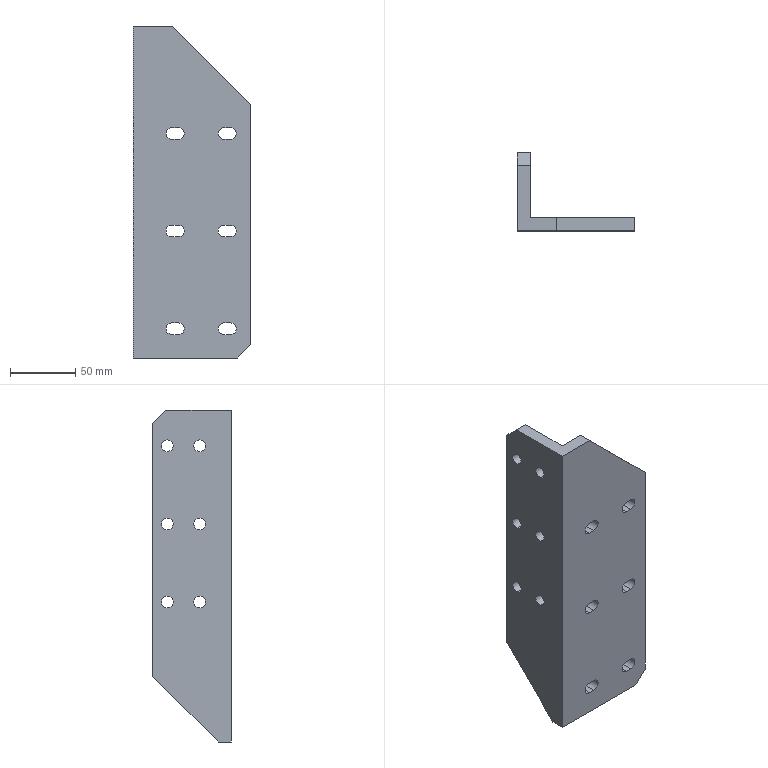Part | SolidWorks | features Chamfer 3, HoleWzd 2, ExtruThin 1 | 1 solid | 48 faces | box 90 x 60 x 255 mm | volume 315166 mm3 | cylinder 24 | plane 24 | commonest cylinder face diameters 9 x24
STEP:
#1=CARTESIAN_POINT('',(-10.,39.,104.5));
#2=VERTEX_POINT('',#1);
#3=CARTESIAN_POINT('',(-10.,39.,95.5));
#4=VERTEX_POINT('',#3);
#5=CARTESIAN_POINT('',(-10.,39.,100.));
#6=DIRECTION('',(1.,0.,0.));
#7=DIRECTION('',(0.,0.,-1.));
#8=AXIS2_PLACEMENT_3D('',#5,#6,#7);
#9=CIRCLE('',#8,4.5);
#10=EDGE_CURVE('',#2,#4,#9,.T.);
#11=ORIENTED_EDGE('',*,*,#10,.F.);
#12=CARTESIAN_POINT('',(0.,39.,104.5));
#13=VERTEX_POINT('',#12);
#14=CARTESIAN_POINT('',(0.,39.,104.5));
#15=DIRECTION('',(1.,0.,0.));
#16=VECTOR('',#15,1000.);
#17=LINE('',#14,#16);
#18=EDGE_CURVE('',#2,#13,#17,.T.);
#19=ORIENTED_EDGE('',*,*,#18,.T.);
#20=CARTESIAN_POINT('',(0.,39.,95.5));
#21=VERTEX_POINT('',#20);
#22=CARTESIAN_POINT('',(0.,39.,100.));
#23=DIRECTION('',(1.,0.,0.));
#24=DIRECTION('',(0.,0.,-1.));
#25=AXIS2_PLACEMENT_3D('',#22,#23,#24);
#26=CIRCLE('',#25,4.5);
#27=EDGE_CURVE('',#13,#21,#26,.T.);
#28=ORIENTED_EDGE('',*,*,#27,.T.);
#29=CARTESIAN_POINT('',(0.,39.,95.5));
#30=DIRECTION('',(1.,0.,0.));
#31=VECTOR('',#30,1000.);
#32=LINE('',#29,#31);
#33=EDGE_CURVE('',#4,#21,#32,.T.);
#34=ORIENTED_EDGE('',*,*,#33,.F.);
#35=EDGE_LOOP('',(#11,#19,#28,#34));
#36=FACE_OUTER_BOUND('',#35,.T.);
#37=CARTESIAN_POINT('',(0.,39.,100.));
#38=DIRECTION('',(1.,0.,0.));
#39=DIRECTION('',(0.,0.,-1.));
#40=AXIS2_PLACEMENT_3D('',#37,#38,#39);
#41=CYLINDRICAL_SURFACE('',#40,4.5);
#42=ADVANCED_FACE('',(#36),#41,.F.);
#43=CARTESIAN_POINT('',(-10.,14.,104.5));
#44=VERTEX_POINT('',#43);
#45=CARTESIAN_POINT('',(-10.,14.,95.5));
#46=VERTEX_POINT('',#45);
#47=CARTESIAN_POINT('',(-10.,14.,100.));
#48=DIRECTION('',(1.,0.,0.));
#49=DIRECTION('',(0.,0.,-1.));
#50=AXIS2_PLACEMENT_3D('',#47,#48,#49);
#51=CIRCLE('',#50,4.5);
#52=EDGE_CURVE('',#44,#46,#51,.T.);
#53=ORIENTED_EDGE('',*,*,#52,.F.);
#54=CARTESIAN_POINT('',(0.,14.,104.5));
#55=VERTEX_POINT('',#54);
#56=CARTESIAN_POINT('',(0.,14.,104.5));
#57=DIRECTION('',(1.,0.,0.));
#58=VECTOR('',#57,1000.);
#59=LINE('',#56,#58);
#60=EDGE_CURVE('',#44,#55,#59,.T.);
#61=ORIENTED_EDGE('',*,*,#60,.T.);
#62=CARTESIAN_POINT('',(0.,14.,95.5));
#63=VERTEX_POINT('',#62);
#64=CARTESIAN_POINT('',(0.,14.,100.));
#65=DIRECTION('',(1.,0.,0.));
#66=DIRECTION('',(0.,0.,-1.));
#67=AXIS2_PLACEMENT_3D('',#64,#65,#66);
#68=CIRCLE('',#67,4.5);
#69=EDGE_CURVE('',#55,#63,#68,.T.);
#70=ORIENTED_EDGE('',*,*,#69,.T.);
#71=CARTESIAN_POINT('',(0.,14.,95.5));
#72=DIRECTION('',(1.,0.,0.));
#73=VECTOR('',#72,1000.);
#74=LINE('',#71,#73);
#75=EDGE_CURVE('',#46,#63,#74,.T.);
#76=ORIENTED_EDGE('',*,*,#75,.F.);
#77=EDGE_LOOP('',(#53,#61,#70,#76));
#78=FACE_OUTER_BOUND('',#77,.T.);
#79=CARTESIAN_POINT('',(0.,14.,100.));
#80=DIRECTION('',(1.,0.,0.));
#81=DIRECTION('',(0.,0.,-1.));
#82=AXIS2_PLACEMENT_3D('',#79,#80,#81);
#83=CYLINDRICAL_SURFACE('',#82,4.5);
#84=ADVANCED_FACE('',(#78),#83,.F.);
#85=CARTESIAN_POINT('',(-10.,39.,44.5));
#86=VERTEX_POINT('',#85);
#87=CARTESIAN_POINT('',(-10.,39.,35.5));
#88=VERTEX_POINT('',#87);
#89=CARTESIAN_POINT('',(-10.,39.,40.));
#90=DIRECTION('',(1.,0.,0.));
#91=DIRECTION('',(0.,0.,-1.));
#92=AXIS2_PLACEMENT_3D('',#89,#90,#91);
#93=CIRCLE('',#92,4.5);
#94=EDGE_CURVE('',#86,#88,#93,.T.);
#95=ORIENTED_EDGE('',*,*,#94,.F.);
#96=CARTESIAN_POINT('',(0.,39.,44.5));
#97=VERTEX_POINT('',#96);
#98=CARTESIAN_POINT('',(0.,39.,44.5));
#99=DIRECTION('',(1.,0.,0.));
#100=VECTOR('',#99,1000.);
#101=LINE('',#98,#100);
#102=EDGE_CURVE('',#86,#97,#101,.T.);
#103=ORIENTED_EDGE('',*,*,#102,.T.);
#104=CARTESIAN_POINT('',(0.,39.,35.5));
#105=VERTEX_POINT('',#104);
#106=CARTESIAN_POINT('',(0.,39.,40.));
#107=DIRECTION('',(1.,0.,0.));
#108=DIRECTION('',(0.,0.,-1.));
#109=AXIS2_PLACEMENT_3D('',#106,#107,#108);
#110=CIRCLE('',#109,4.5);
#111=EDGE_CURVE('',#97,#105,#110,.T.);
#112=ORIENTED_EDGE('',*,*,#111,.T.);
#113=CARTESIAN_POINT('',(0.,39.,35.5));
#114=DIRECTION('',(1.,0.,0.));
#115=VECTOR('',#114,1000.);
#116=LINE('',#113,#115);
#117=EDGE_CURVE('',#88,#105,#116,.T.);
#118=ORIENTED_EDGE('',*,*,#117,.F.);
#119=EDGE_LOOP('',(#95,#103,#112,#118));
#120=FACE_OUTER_BOUND('',#119,.T.);
#121=CARTESIAN_POINT('',(0.,39.,40.));
#122=DIRECTION('',(1.,0.,0.));
#123=DIRECTION('',(0.,0.,-1.));
#124=AXIS2_PLACEMENT_3D('',#121,#122,#123);
#125=CYLINDRICAL_SURFACE('',#124,4.5);
#126=ADVANCED_FACE('',(#120),#125,.F.);
#127=CARTESIAN_POINT('',(-10.,14.,44.5));
#128=VERTEX_POINT('',#127);
#129=CARTESIAN_POINT('',(-10.,14.,35.5));
#130=VERTEX_POINT('',#129);
#131=CARTESIAN_POINT('',(-10.,14.,40.));
#132=DIRECTION('',(1.,0.,0.));
#133=DIRECTION('',(0.,0.,-1.));
#134=AXIS2_PLACEMENT_3D('',#131,#132,#133);
#135=CIRCLE('',#134,4.5);
#136=EDGE_CURVE('',#128,#130,#135,.T.);
#137=ORIENTED_EDGE('',*,*,#136,.F.);
#138=CARTESIAN_POINT('',(0.,14.,44.5));
#139=VERTEX_POINT('',#138);
#140=CARTESIAN_POINT('',(0.,14.,44.5));
#141=DIRECTION('',(1.,0.,0.));
#142=VECTOR('',#141,1000.);
#143=LINE('',#140,#142);
#144=EDGE_CURVE('',#128,#139,#143,.T.);
#145=ORIENTED_EDGE('',*,*,#144,.T.);
#146=CARTESIAN_POINT('',(0.,14.,35.5));
#147=VERTEX_POINT('',#146);
#148=CARTESIAN_POINT('',(0.,14.,40.));
#149=DIRECTION('',(1.,0.,0.));
#150=DIRECTION('',(0.,0.,-1.));
#151=AXIS2_PLACEMENT_3D('',#148,#149,#150);
#152=CIRCLE('',#151,4.5);
#153=EDGE_CURVE('',#139,#147,#152,.T.);
#154=ORIENTED_EDGE('',*,*,#153,.T.);
#155=CARTESIAN_POINT('',(0.,14.,35.5));
#156=DIRECTION('',(1.,0.,0.));
#157=VECTOR('',#156,1000.);
#158=LINE('',#155,#157);
#159=EDGE_CURVE('',#130,#147,#158,.T.);
#160=ORIENTED_EDGE('',*,*,#159,.F.);
#161=EDGE_LOOP('',(#137,#145,#154,#160));
#162=FACE_OUTER_BOUND('',#161,.T.);
#163=CARTESIAN_POINT('',(0.,14.,40.));
#164=DIRECTION('',(1.,0.,0.));
#165=DIRECTION('',(0.,0.,-1.));
#166=AXIS2_PLACEMENT_3D('',#163,#164,#165);
#167=CYLINDRICAL_SURFACE('',#166,4.5);
#168=ADVANCED_FACE('',(#162),#167,.F.);
#169=CARTESIAN_POINT('',(-10.,39.,-15.5));
#170=VERTEX_POINT('',#169);
#171=CARTESIAN_POINT('',(-10.,39.,-24.5));
#172=VERTEX_POINT('',#171);
#173=CARTESIAN_POINT('',(-10.,39.,-20.));
#174=DIRECTION('',(1.,0.,0.));
#175=DIRECTION('',(0.,0.,-1.));
#176=AXIS2_PLACEMENT_3D('',#173,#174,#175);
#177=CIRCLE('',#176,4.5);
#178=EDGE_CURVE('',#170,#172,#177,.T.);
#179=ORIENTED_EDGE('',*,*,#178,.F.);
#180=CARTESIAN_POINT('',(0.,39.,-15.5));
#181=VERTEX_POINT('',#180);
#182=CARTESIAN_POINT('',(0.,39.,-15.5));
#183=DIRECTION('',(1.,0.,0.));
#184=VECTOR('',#183,1000.);
#185=LINE('',#182,#184);
#186=EDGE_CURVE('',#170,#181,#185,.T.);
#187=ORIENTED_EDGE('',*,*,#186,.T.);
#188=CARTESIAN_POINT('',(0.,39.,-24.5));
#189=VERTEX_POINT('',#188);
#190=CARTESIAN_POINT('',(0.,39.,-20.));
#191=DIRECTION('',(1.,0.,0.));
#192=DIRECTION('',(0.,0.,-1.));
#193=AXIS2_PLACEMENT_3D('',#190,#191,#192);
#194=CIRCLE('',#193,4.5);
#195=EDGE_CURVE('',#181,#189,#194,.T.);
#196=ORIENTED_EDGE('',*,*,#195,.T.);
#197=CARTESIAN_POINT('',(0.,39.,-24.5));
#198=DIRECTION('',(1.,0.,0.));
#199=VECTOR('',#198,1000.);
#200=LINE('',#197,#199);
#201=EDGE_CURVE('',#172,#189,#200,.T.);
#202=ORIENTED_EDGE('',*,*,#201,.F.);
#203=EDGE_LOOP('',(#179,#187,#196,#202));
#204=FACE_OUTER_BOUND('',#203,.T.);
#205=CARTESIAN_POINT('',(0.,39.,-20.));
#206=DIRECTION('',(1.,0.,0.));
#207=DIRECTION('',(0.,0.,-1.));
#208=AXIS2_PLACEMENT_3D('',#205,#206,#207);
#209=CYLINDRICAL_SURFACE('',#208,4.5);
#210=ADVANCED_FACE('',(#204),#209,.F.);
#211=CARTESIAN_POINT('',(-10.,14.,-15.5));
#212=VERTEX_POINT('',#211);
#213=CARTESIAN_POINT('',(-10.,14.,-24.5));
#214=VERTEX_POINT('',#213);
#215=CARTESIAN_POINT('',(-10.,14.,-20.));
#216=DIRECTION('',(1.,0.,0.));
#217=DIRECTION('',(0.,0.,-1.));
#218=AXIS2_PLACEMENT_3D('',#215,#216,#217);
#219=CIRCLE('',#218,4.5);
#220=EDGE_CURVE('',#212,#214,#219,.T.);
#221=ORIENTED_EDGE('',*,*,#220,.F.);
#222=CARTESIAN_POINT('',(0.,14.,-15.5));
#223=VERTEX_POINT('',#222);
#224=CARTESIAN_POINT('',(0.,14.,-15.5));
#225=DIRECTION('',(1.,0.,0.));
#226=VECTOR('',#225,1000.);
#227=LINE('',#224,#226);
#228=EDGE_CURVE('',#212,#223,#227,.T.);
#229=ORIENTED_EDGE('',*,*,#228,.T.);
#230=CARTESIAN_POINT('',(0.,14.,-24.5));
#231=VERTEX_POINT('',#230);
#232=CARTESIAN_POINT('',(0.,14.,-20.));
#233=DIRECTION('',(1.,0.,0.));
#234=DIRECTION('',(0.,0.,-1.));
#235=AXIS2_PLACEMENT_3D('',#232,#233,#234);
#236=CIRCLE('',#235,4.5);
#237=EDGE_CURVE('',#223,#231,#236,.T.);
#238=ORIENTED_EDGE('',*,*,#237,.T.);
#239=CARTESIAN_POINT('',(0.,14.,-24.5));
#240=DIRECTION('',(1.,0.,0.));
#241=VECTOR('',#240,1000.);
#242=LINE('',#239,#241);
#243=EDGE_CURVE('',#214,#231,#242,.T.);
#244=ORIENTED_EDGE('',*,*,#243,.F.);
#245=EDGE_LOOP('',(#221,#229,#238,#244));
#246=FACE_OUTER_BOUND('',#245,.T.);
#247=CARTESIAN_POINT('',(0.,14.,-20.));
#248=DIRECTION('',(1.,0.,0.));
#249=DIRECTION('',(0.,0.,-1.));
#250=AXIS2_PLACEMENT_3D('',#247,#248,#249);
#251=CYLINDRICAL_SURFACE('',#250,4.5);
#252=ADVANCED_FACE('',(#246),#251,.F.);
#253=CARTESIAN_POINT('',(59.5,-10.,-109.5));
#254=VERTEX_POINT('',#253);
#255=CARTESIAN_POINT('',(64.5,-10.,-109.5));
#256=VERTEX_POINT('',#255);
#257=CARTESIAN_POINT('',(59.5,-10.,-109.5));
#258=DIRECTION('',(1.,0.,0.));
#259=VECTOR('',#258,1000.);
#260=LINE('',#257,#259);
#261=EDGE_CURVE('',#254,#256,#260,.T.);
#262=ORIENTED_EDGE('',*,*,#261,.F.);
#263=CARTESIAN_POINT('',(59.5,-10.,-100.5));
#264=VERTEX_POINT('',#263);
#265=CARTESIAN_POINT('',(59.5,-10.,-105.));
#266=DIRECTION('',(0.,1.,0.));
#267=DIRECTION('',(0.,0.,1.));
#268=AXIS2_PLACEMENT_3D('',#265,#266,#267);
#269=CIRCLE('',#268,4.5);
#270=EDGE_CURVE('',#254,#264,#269,.T.);
#271=ORIENTED_EDGE('',*,*,#270,.T.);
#272=CARTESIAN_POINT('',(64.5,-10.,-100.5));
#273=VERTEX_POINT('',#272);
#274=CARTESIAN_POINT('',(59.5,-10.,-100.5));
#275=DIRECTION('',(1.,0.,0.));
#276=VECTOR('',#275,1000.);
#277=LINE('',#274,#276);
#278=EDGE_CURVE('',#264,#273,#277,.T.);
#279=ORIENTED_EDGE('',*,*,#278,.T.);
#280=CARTESIAN_POINT('',(64.5,-10.,-105.));
#281=DIRECTION('',(0.,1.,0.));
#282=DIRECTION('',(0.,0.,1.));
#283=AXIS2_PLACEMENT_3D('',#280,#281,#282);
#284=CIRCLE('',#283,4.5);
#285=EDGE_CURVE('',#273,#256,#284,.T.);
#286=ORIENTED_EDGE('',*,*,#285,.T.);
#287=EDGE_LOOP('',(#262,#271,#279,#286));
#288=FACE_BOUND('',#287,.T.);
#289=CARTESIAN_POINT('',(64.5,-10.,-25.5));
#290=VERTEX_POINT('',#289);
#291=CARTESIAN_POINT('',(64.5,-10.,-34.5));
#292=VERTEX_POINT('',#291);
#293=CARTESIAN_POINT('',(64.5,-10.,-30.));
#294=DIRECTION('',(0.,1.,0.));
#295=DIRECTION('',(0.,0.,1.));
#296=AXIS2_PLACEMENT_3D('',#293,#294,#295);
#297=CIRCLE('',#296,4.5);
#298=EDGE_CURVE('',#290,#292,#297,.T.);
#299=ORIENTED_EDGE('',*,*,#298,.T.);
#300=CARTESIAN_POINT('',(59.5,-10.,-34.5));
#301=VERTEX_POINT('',#300);
#302=CARTESIAN_POINT('',(59.5,-10.,-34.5));
#303=DIRECTION('',(1.,0.,0.));
#304=VECTOR('',#303,1000.);
#305=LINE('',#302,#304);
#306=EDGE_CURVE('',#301,#292,#305,.T.);
#307=ORIENTED_EDGE('',*,*,#306,.F.);
#308=CARTESIAN_POINT('',(59.5,-10.,-25.5));
#309=VERTEX_POINT('',#308);
#310=CARTESIAN_POINT('',(59.5,-10.,-30.));
#311=DIRECTION('',(0.,1.,0.));
#312=DIRECTION('',(0.,0.,1.));
#313=AXIS2_PLACEMENT_3D('',#310,#311,#312);
#314=CIRCLE('',#313,4.5);
#315=EDGE_CURVE('',#301,#309,#314,.T.);
#316=ORIENTED_EDGE('',*,*,#315,.T.);
#317=CARTESIAN_POINT('',(59.5,-10.,-25.5));
#318=DIRECTION('',(1.,0.,0.));
#319=VECTOR('',#318,1000.);
#320=LINE('',#317,#319);
#321=EDGE_CURVE('',#309,#290,#320,.T.);
#322=ORIENTED_EDGE('',*,*,#321,.T.);
#323=EDGE_LOOP('',(#299,#307,#316,#322));
#324=FACE_BOUND('',#323,.T.);
#325=CARTESIAN_POINT('',(19.5,-10.,-109.5));
#326=VERTEX_POINT('',#325);
#327=CARTESIAN_POINT('',(24.5,-10.,-109.5));
#328=VERTEX_POINT('',#327);
#329=CARTESIAN_POINT('',(19.5,-10.,-109.5));
#330=DIRECTION('',(1.,0.,0.));
#331=VECTOR('',#330,1000.);
#332=LINE('',#329,#331);
#333=EDGE_CURVE('',#326,#328,#332,.T.);
#334=ORIENTED_EDGE('',*,*,#333,.F.);
#335=CARTESIAN_POINT('',(19.5,-10.,-100.5));
#336=VERTEX_POINT('',#335);
#337=CARTESIAN_POINT('',(19.5,-10.,-105.));
#338=DIRECTION('',(0.,1.,0.));
#339=DIRECTION('',(0.,0.,1.));
#340=AXIS2_PLACEMENT_3D('',#337,#338,#339);
#341=CIRCLE('',#340,4.5);
#342=EDGE_CURVE('',#326,#336,#341,.T.);
#343=ORIENTED_EDGE('',*,*,#342,.T.);
#344=CARTESIAN_POINT('',(24.5,-10.,-100.5));
#345=VERTEX_POINT('',#344);
#346=CARTESIAN_POINT('',(19.5,-10.,-100.5));
#347=DIRECTION('',(1.,0.,0.));
#348=VECTOR('',#347,1000.);
#349=LINE('',#346,#348);
#350=EDGE_CURVE('',#336,#345,#349,.T.);
#351=ORIENTED_EDGE('',*,*,#350,.T.);
#352=CARTESIAN_POINT('',(24.5,-10.,-105.));
#353=DIRECTION('',(0.,1.,0.));
#354=DIRECTION('',(0.,0.,1.));
#355=AXIS2_PLACEMENT_3D('',#352,#353,#354);
#356=CIRCLE('',#355,4.5);
#357=EDGE_CURVE('',#345,#328,#356,.T.);
#358=ORIENTED_EDGE('',*,*,#357,.T.);
#359=EDGE_LOOP('',(#334,#343,#351,#358));
#360=FACE_BOUND('',#359,.T.);
#361=CARTESIAN_POINT('',(19.5,-10.,-34.5));
#362=VERTEX_POINT('',#361);
#363=CARTESIAN_POINT('',(24.5,-10.,-34.5));
#364=VERTEX_POINT('',#363);
#365=CARTESIAN_POINT('',(19.5,-10.,-34.5));
#366=DIRECTION('',(1.,0.,0.));
#367=VECTOR('',#366,1000.);
#368=LINE('',#365,#367);
#369=EDGE_CURVE('',#362,#364,#368,.T.);
#370=ORIENTED_EDGE('',*,*,#369,.F.);
#371=CARTESIAN_POINT('',(19.5,-10.,-25.5));
#372=VERTEX_POINT('',#371);
#373=CARTESIAN_POINT('',(19.5,-10.,-30.));
#374=DIRECTION('',(0.,1.,0.));
#375=DIRECTION('',(0.,0.,1.));
#376=AXIS2_PLACEMENT_3D('',#373,#374,#375);
#377=CIRCLE('',#376,4.5);
#378=EDGE_CURVE('',#362,#372,#377,.T.);
#379=ORIENTED_EDGE('',*,*,#378,.T.);
#380=CARTESIAN_POINT('',(24.5,-10.,-25.5));
#381=VERTEX_POINT('',#380);
#382=CARTESIAN_POINT('',(19.5,-10.,-25.5));
#383=DIRECTION('',(1.,0.,0.));
#384=VECTOR('',#383,1000.);
#385=LINE('',#382,#384);
#386=EDGE_CURVE('',#372,#381,#385,.T.);
#387=ORIENTED_EDGE('',*,*,#386,.T.);
#388=CARTESIAN_POINT('',(24.5,-10.,-30.));
#389=DIRECTION('',(0.,1.,0.));
#390=DIRECTION('',(0.,0.,1.));
#391=AXIS2_PLACEMENT_3D('',#388,#389,#390);
#392=CIRCLE('',#391,4.5);
#393=EDGE_CURVE('',#381,#364,#392,.T.);
#394=ORIENTED_EDGE('',*,*,#393,.T.);
#395=EDGE_LOOP('',(#370,#379,#387,#394));
#396=FACE_BOUND('',#395,.T.);
#397=CARTESIAN_POINT('',(19.5,-10.,40.5));
#398=VERTEX_POINT('',#397);
#399=CARTESIAN_POINT('',(19.5,-10.,49.5));
#400=VERTEX_POINT('',#399);
#401=CARTESIAN_POINT('',(19.5,-10.,45.));
#402=DIRECTION('',(0.,1.,0.));
#403=DIRECTION('',(0.,0.,1.));
#404=AXIS2_PLACEMENT_3D('',#401,#402,#403);
#405=CIRCLE('',#404,4.5);
#406=EDGE_CURVE('',#398,#400,#405,.T.);
#407=ORIENTED_EDGE('',*,*,#406,.T.);
#408=CARTESIAN_POINT('',(24.5,-10.,49.5));
#409=VERTEX_POINT('',#408);
#410=CARTESIAN_POINT('',(19.5,-10.,49.5));
#411=DIRECTION('',(1.,0.,0.));
#412=VECTOR('',#411,1000.);
#413=LINE('',#410,#412);
#414=EDGE_CURVE('',#400,#409,#413,.T.);
#415=ORIENTED_EDGE('',*,*,#414,.T.);
#416=CARTESIAN_POINT('',(24.5,-10.,40.5));
#417=VERTEX_POINT('',#416);
#418=CARTESIAN_POINT('',(24.5,-10.,45.));
#419=DIRECTION('',(0.,1.,0.));
#420=DIRECTION('',(0.,0.,1.));
#421=AXIS2_PLACEMENT_3D('',#418,#419,#420);
#422=CIRCLE('',#421,4.5);
#423=EDGE_CURVE('',#409,#417,#422,.T.);
#424=ORIENTED_EDGE('',*,*,#423,.T.);
#425=CARTESIAN_POINT('',(19.5,-10.,40.5));
#426=DIRECTION('',(1.,0.,0.));
#427=VECTOR('',#426,1000.);
#428=LINE('',#425,#427);
#429=EDGE_CURVE('',#398,#417,#428,.T.);
#430=ORIENTED_EDGE('',*,*,#429,.F.);
#431=EDGE_LOOP('',(#407,#415,#424,#430));
#432=FACE_BOUND('',#431,.T.);
#433=CARTESIAN_POINT('',(-10.,-10.,-127.5));
#434=VERTEX_POINT('',#433);
#435=CARTESIAN_POINT('',(70.,-10.,-127.5));
#436=VERTEX_POINT('',#435);
#437=CARTESIAN_POINT('',(0.,-10.,-127.5));
#438=DIRECTION('',(1.,0.,0.));
#439=VECTOR('',#438,1000.);
#440=LINE('',#437,#439);
#441=EDGE_CURVE('',#434,#436,#440,.T.);
#442=ORIENTED_EDGE('',*,*,#441,.T.);
#443=CARTESIAN_POINT('',(80.,-10.,-117.5));
#444=VERTEX_POINT('',#443);
#445=CARTESIAN_POINT('',(70.,-10.,-127.5));
#446=DIRECTION('',(0.7071,0.,0.7071));
#447=VECTOR('',#446,1000.);
#448=LINE('',#445,#447);
#449=EDGE_CURVE('',#436,#444,#448,.T.);
#450=ORIENTED_EDGE('',*,*,#449,.T.);
#451=CARTESIAN_POINT('',(80.,-10.,67.5));
#452=VERTEX_POINT('',#451);
#453=CARTESIAN_POINT('',(80.,-10.,127.5));
#454=DIRECTION('',(0.,0.,-1.));
#455=VECTOR('',#454,1000.);
#456=LINE('',#453,#455);
#457=EDGE_CURVE('',#452,#444,#456,.T.);
#458=ORIENTED_EDGE('',*,*,#457,.F.);
#459=CARTESIAN_POINT('',(20.,-10.,127.5));
#460=VERTEX_POINT('',#459);
#461=CARTESIAN_POINT('',(80.,-10.,67.5));
#462=DIRECTION('',(-0.7071,0.,0.7071));
#463=VECTOR('',#462,1000.);
#464=LINE('',#461,#463);
#465=EDGE_CURVE('',#452,#460,#464,.T.);
#466=ORIENTED_EDGE('',*,*,#465,.T.);
#467=CARTESIAN_POINT('',(-10.,-10.,127.5));
#468=VERTEX_POINT('',#467);
#469=CARTESIAN_POINT('',(0.,-10.,127.5));
#470=DIRECTION('',(1.,0.,0.));
#471=VECTOR('',#470,1000.);
#472=LINE('',#469,#471);
#473=EDGE_CURVE('',#468,#460,#472,.T.);
#474=ORIENTED_EDGE('',*,*,#473,.F.);
#475=CARTESIAN_POINT('',(-10.,-10.,127.5));
#476=DIRECTION('',(0.,0.,-1.));
#477=VECTOR('',#476,1000.);
#478=LINE('',#475,#477);
#479=EDGE_CURVE('',#468,#434,#478,.T.);
#480=ORIENTED_EDGE('',*,*,#479,.T.);
#481=EDGE_LOOP('',(#442,#450,#458,#466,#474,#480));
#482=FACE_OUTER_BOUND('',#481,.T.);
#483=CARTESIAN_POINT('',(59.5,-10.,40.5));
#484=VERTEX_POINT('',#483);
#485=CARTESIAN_POINT('',(64.5,-10.,40.5));
#486=VERTEX_POINT('',#485);
#487=CARTESIAN_POINT('',(59.5,-10.,40.5));
#488=DIRECTION('',(1.,0.,0.));
#489=VECTOR('',#488,1000.);
#490=LINE('',#487,#489);
#491=EDGE_CURVE('',#484,#486,#490,.T.);
#492=ORIENTED_EDGE('',*,*,#491,.F.);
#493=CARTESIAN_POINT('',(59.5,-10.,49.5));
#494=VERTEX_POINT('',#493);
#495=CARTESIAN_POINT('',(59.5,-10.,45.));
#496=DIRECTION('',(0.,1.,0.));
#497=DIRECTION('',(0.,0.,1.));
#498=AXIS2_PLACEMENT_3D('',#495,#496,#497);
#499=CIRCLE('',#498,4.5);
#500=EDGE_CURVE('',#484,#494,#499,.T.);
#501=ORIENTED_EDGE('',*,*,#500,.T.);
#502=CARTESIAN_POINT('',(64.5,-10.,49.5));
#503=VERTEX_POINT('',#502);
#504=CARTESIAN_POINT('',(59.5,-10.,49.5));
#505=DIRECTION('',(1.,0.,0.));
#506=VECTOR('',#505,1000.);
#507=LINE('',#504,#506);
#508=EDGE_CURVE('',#494,#503,#507,.T.);
#509=ORIENTED_EDGE('',*,*,#508,.T.);
#510=CARTESIAN_POINT('',(64.5,-10.,45.));
#511=DIRECTION('',(0.,1.,0.));
#512=DIRECTION('',(0.,0.,1.));
#513=AXIS2_PLACEMENT_3D('',#510,#511,#512);
#514=CIRCLE('',#513,4.5);
#515=EDGE_CURVE('',#503,#486,#514,.T.);
#516=ORIENTED_EDGE('',*,*,#515,.T.);
#517=EDGE_LOOP('',(#492,#501,#509,#516));
#518=FACE_BOUND('',#517,.T.);
#519=CARTESIAN_POINT('',(0.,-10.,127.5));
#520=DIRECTION('',(0.,1.,0.));
#521=DIRECTION('',(0.,0.,1.));
#522=AXIS2_PLACEMENT_3D('',#519,#520,#521);
#523=PLANE('',#522);
#524=ADVANCED_FACE('',(#288,#324,#360,#396,#432,#482,#518),#523,.F.);
#525=ORIENTED_EDGE('',*,*,#457,.T.);
#526=CARTESIAN_POINT('',(80.,0.,-117.5));
#527=VERTEX_POINT('',#526);
#528=CARTESIAN_POINT('',(80.,0.,-117.5));
#529=DIRECTION('',(0.,1.,0.));
#530=VECTOR('',#529,1000.);
#531=LINE('',#528,#530);
#532=EDGE_CURVE('',#444,#527,#531,.T.);
#533=ORIENTED_EDGE('',*,*,#532,.T.);
#534=CARTESIAN_POINT('',(80.,0.,67.5));
#535=VERTEX_POINT('',#534);
#536=CARTESIAN_POINT('',(80.,0.,127.5));
#537=DIRECTION('',(0.,0.,-1.));
#538=VECTOR('',#537,1000.);
#539=LINE('',#536,#538);
#540=EDGE_CURVE('',#535,#527,#539,.T.);
#541=ORIENTED_EDGE('',*,*,#540,.F.);
#542=CARTESIAN_POINT('',(80.,-10.,67.5));
#543=DIRECTION('',(0.,-1.,0.));
#544=VECTOR('',#543,1000.);
#545=LINE('',#542,#544);
#546=EDGE_CURVE('',#535,#452,#545,.T.);
#547=ORIENTED_EDGE('',*,*,#546,.T.);
#548=EDGE_LOOP('',(#525,#533,#541,#547));
#549=FACE_OUTER_BOUND('',#548,.T.);
#550=CARTESIAN_POINT('',(80.,0.,127.5));
#551=DIRECTION('',(1.,0.,0.));
#552=DIRECTION('',(0.,0.,-1.));
#553=AXIS2_PLACEMENT_3D('',#550,#551,#552);
#554=PLANE('',#553);
#555=ADVANCED_FACE('',(#549),#554,.T.);
#556=CARTESIAN_POINT('',(64.5,0.,-100.5));
#557=VERTEX_POINT('',#556);
#558=CARTESIAN_POINT('',(64.5,0.,-109.5));
#559=VERTEX_POINT('',#558);
#560=CARTESIAN_POINT('',(64.5,0.,-105.));
#561=DIRECTION('',(0.,1.,0.));
#562=DIRECTION('',(0.,0.,1.));
#563=AXIS2_PLACEMENT_3D('',#560,#561,#562);
#564=CIRCLE('',#563,4.5);
#565=EDGE_CURVE('',#557,#559,#564,.T.);
#566=ORIENTED_EDGE('',*,*,#565,.F.);
#567=CARTESIAN_POINT('',(59.5,0.,-100.5));
#568=VERTEX_POINT('',#567);
#569=CARTESIAN_POINT('',(59.5,0.,-100.5));
#570=DIRECTION('',(1.,0.,0.));
#571=VECTOR('',#570,1000.);
#572=LINE('',#569,#571);
#573=EDGE_CURVE('',#568,#557,#572,.T.);
#574=ORIENTED_EDGE('',*,*,#573,.F.);
#575=CARTESIAN_POINT('',(59.5,0.,-109.5));
#576=VERTEX_POINT('',#575);
#577=CARTESIAN_POINT('',(59.5,0.,-105.));
#578=DIRECTION('',(0.,1.,0.));
#579=DIRECTION('',(0.,0.,1.));
#580=AXIS2_PLACEMENT_3D('',#577,#578,#579);
#581=CIRCLE('',#580,4.5);
#582=EDGE_CURVE('',#576,#568,#581,.T.);
#583=ORIENTED_EDGE('',*,*,#582,.F.);
#584=CARTESIAN_POINT('',(59.5,0.,-109.5));
#585=DIRECTION('',(1.,0.,0.));
#586=VECTOR('',#585,1000.);
#587=LINE('',#584,#586);
#588=EDGE_CURVE('',#576,#559,#587,.T.);
#589=ORIENTED_EDGE('',*,*,#588,.T.);
#590=EDGE_LOOP('',(#566,#574,#583,#589));
#591=FACE_BOUND('',#590,.T.);
#592=CARTESIAN_POINT('',(64.5,0.,-25.5));
#593=VERTEX_POINT('',#592);
#594=CARTESIAN_POINT('',(64.5,0.,-34.5));
#595=VERTEX_POINT('',#594);
#596=CARTESIAN_POINT('',(64.5,0.,-30.));
#597=DIRECTION('',(0.,1.,0.));
#598=DIRECTION('',(0.,0.,1.));
#599=AXIS2_PLACEMENT_3D('',#596,#597,#598);
#600=CIRCLE('',#599,4.5);
#601=EDGE_CURVE('',#593,#595,#600,.T.);
#602=ORIENTED_EDGE('',*,*,#601,.F.);
#603=CARTESIAN_POINT('',(59.5,0.,-25.5));
#604=VERTEX_POINT('',#603);
#605=CARTESIAN_POINT('',(59.5,0.,-25.5));
#606=DIRECTION('',(1.,0.,0.));
#607=VECTOR('',#606,1000.);
#608=LINE('',#605,#607);
#609=EDGE_CURVE('',#604,#593,#608,.T.);
#610=ORIENTED_EDGE('',*,*,#609,.F.);
#611=CARTESIAN_POINT('',(59.5,0.,-34.5));
#612=VERTEX_POINT('',#611);
#613=CARTESIAN_POINT('',(59.5,0.,-30.));
#614=DIRECTION('',(0.,1.,0.));
#615=DIRECTION('',(0.,0.,1.));
#616=AXIS2_PLACEMENT_3D('',#613,#614,#615);
#617=CIRCLE('',#616,4.5);
#618=EDGE_CURVE('',#612,#604,#617,.T.);
#619=ORIENTED_EDGE('',*,*,#618,.F.);
#620=CARTESIAN_POINT('',(59.5,0.,-34.5));
#621=DIRECTION('',(1.,0.,0.));
#622=VECTOR('',#621,1000.);
#623=LINE('',#620,#622);
#624=EDGE_CURVE('',#612,#595,#623,.T.);
#625=ORIENTED_EDGE('',*,*,#624,.T.);
#626=EDGE_LOOP('',(#602,#610,#619,#625));
#627=FACE_BOUND('',#626,.T.);
#628=CARTESIAN_POINT('',(64.5,0.,49.5));
#629=VERTEX_POINT('',#628);
#630=CARTESIAN_POINT('',(64.5,0.,40.5));
#631=VERTEX_POINT('',#630);
#632=CARTESIAN_POINT('',(64.5,0.,45.));
#633=DIRECTION('',(0.,1.,0.));
#634=DIRECTION('',(0.,0.,1.));
#635=AXIS2_PLACEMENT_3D('',#632,#633,#634);
#636=CIRCLE('',#635,4.5);
#637=EDGE_CURVE('',#629,#631,#636,.T.);
#638=ORIENTED_EDGE('',*,*,#637,.F.);
#639=CARTESIAN_POINT('',(59.5,0.,49.5));
#640=VERTEX_POINT('',#639);
#641=CARTESIAN_POINT('',(59.5,0.,49.5));
#642=DIRECTION('',(1.,0.,0.));
#643=VECTOR('',#642,1000.);
#644=LINE('',#641,#643);
#645=EDGE_CURVE('',#640,#629,#644,.T.);
#646=ORIENTED_EDGE('',*,*,#645,.F.);
#647=CARTESIAN_POINT('',(59.5,0.,40.5));
#648=VERTEX_POINT('',#647);
#649=CARTESIAN_POINT('',(59.5,0.,45.));
#650=DIRECTION('',(0.,1.,0.));
#651=DIRECTION('',(0.,0.,1.));
#652=AXIS2_PLACEMENT_3D('',#649,#650,#651);
#653=CIRCLE('',#652,4.5);
#654=EDGE_CURVE('',#648,#640,#653,.T.);
#655=ORIENTED_EDGE('',*,*,#654,.F.);
#656=CARTESIAN_POINT('',(59.5,0.,40.5));
#657=DIRECTION('',(1.,0.,0.));
#658=VECTOR('',#657,1000.);
#659=LINE('',#656,#658);
#660=EDGE_CURVE('',#648,#631,#659,.T.);
#661=ORIENTED_EDGE('',*,*,#660,.T.);
#662=EDGE_LOOP('',(#638,#646,#655,#661));
#663=FACE_BOUND('',#662,.T.);
#664=CARTESIAN_POINT('',(24.5,0.,-100.5));
#665=VERTEX_POINT('',#664);
#666=CARTESIAN_POINT('',(24.5,0.,-109.5));
#667=VERTEX_POINT('',#666);
#668=CARTESIAN_POINT('',(24.5,0.,-105.));
#669=DIRECTION('',(0.,1.,0.));
#670=DIRECTION('',(0.,0.,1.));
#671=AXIS2_PLACEMENT_3D('',#668,#669,#670);
#672=CIRCLE('',#671,4.5);
#673=EDGE_CURVE('',#665,#667,#672,.T.);
#674=ORIENTED_EDGE('',*,*,#673,.F.);
#675=CARTESIAN_POINT('',(19.5,0.,-100.5));
#676=VERTEX_POINT('',#675);
#677=CARTESIAN_POINT('',(19.5,0.,-100.5));
#678=DIRECTION('',(1.,0.,0.));
#679=VECTOR('',#678,1000.);
#680=LINE('',#677,#679);
#681=EDGE_CURVE('',#676,#665,#680,.T.);
#682=ORIENTED_EDGE('',*,*,#681,.F.);
#683=CARTESIAN_POINT('',(19.5,0.,-109.5));
#684=VERTEX_POINT('',#683);
#685=CARTESIAN_POINT('',(19.5,0.,-105.));
#686=DIRECTION('',(0.,1.,0.));
#687=DIRECTION('',(0.,0.,1.));
#688=AXIS2_PLACEMENT_3D('',#685,#686,#687);
#689=CIRCLE('',#688,4.5);
#690=EDGE_CURVE('',#684,#676,#689,.T.);
#691=ORIENTED_EDGE('',*,*,#690,.F.);
#692=CARTESIAN_POINT('',(19.5,0.,-109.5));
#693=DIRECTION('',(1.,0.,0.));
#694=VECTOR('',#693,1000.);
#695=LINE('',#692,#694);
#696=EDGE_CURVE('',#684,#667,#695,.T.);
#697=ORIENTED_EDGE('',*,*,#696,.T.);
#698=EDGE_LOOP('',(#674,#682,#691,#697));
#699=FACE_BOUND('',#698,.T.);
#700=CARTESIAN_POINT('',(19.5,0.,-34.5));
#701=VERTEX_POINT('',#700);
#702=CARTESIAN_POINT('',(24.5,0.,-34.5));
#703=VERTEX_POINT('',#702);
#704=CARTESIAN_POINT('',(19.5,0.,-34.5));
#705=DIRECTION('',(1.,0.,0.));
#706=VECTOR('',#705,1000.);
#707=LINE('',#704,#706);
#708=EDGE_CURVE('',#701,#703,#707,.T.);
#709=ORIENTED_EDGE('',*,*,#708,.T.);
#710=CARTESIAN_POINT('',(24.5,0.,-25.5));
#711=VERTEX_POINT('',#710);
#712=CARTESIAN_POINT('',(24.5,0.,-30.));
#713=DIRECTION('',(0.,1.,0.));
#714=DIRECTION('',(0.,0.,1.));
#715=AXIS2_PLACEMENT_3D('',#712,#713,#714);
#716=CIRCLE('',#715,4.5);
#717=EDGE_CURVE('',#711,#703,#716,.T.);
#718=ORIENTED_EDGE('',*,*,#717,.F.);
#719=CARTESIAN_POINT('',(19.5,0.,-25.5));
#720=VERTEX_POINT('',#719);
#721=CARTESIAN_POINT('',(19.5,0.,-25.5));
#722=DIRECTION('',(1.,0.,0.));
#723=VECTOR('',#722,1000.);
#724=LINE('',#721,#723);
#725=EDGE_CURVE('',#720,#711,#724,.T.);
#726=ORIENTED_EDGE('',*,*,#725,.F.);
#727=CARTESIAN_POINT('',(19.5,0.,-30.));
#728=DIRECTION('',(0.,1.,0.));
#729=DIRECTION('',(0.,0.,1.));
#730=AXIS2_PLACEMENT_3D('',#727,#728,#729);
#731=CIRCLE('',#730,4.5);
#732=EDGE_CURVE('',#701,#720,#731,.T.);
#733=ORIENTED_EDGE('',*,*,#732,.F.);
#734=EDGE_LOOP('',(#709,#718,#726,#733));
#735=FACE_BOUND('',#734,.T.);
#736=CARTESIAN_POINT('',(24.5,0.,49.5));
#737=VERTEX_POINT('',#736);
#738=CARTESIAN_POINT('',(24.5,0.,40.5));
#739=VERTEX_POINT('',#738);
#740=CARTESIAN_POINT('',(24.5,0.,45.));
#741=DIRECTION('',(0.,1.,0.));
#742=DIRECTION('',(0.,0.,1.));
#743=AXIS2_PLACEMENT_3D('',#740,#741,#742);
#744=CIRCLE('',#743,4.5);
#745=EDGE_CURVE('',#737,#739,#744,.T.);
#746=ORIENTED_EDGE('',*,*,#745,.F.);
#747=CARTESIAN_POINT('',(19.5,0.,49.5));
#748=VERTEX_POINT('',#747);
#749=CARTESIAN_POINT('',(19.5,0.,49.5));
#750=DIRECTION('',(1.,0.,0.));
#751=VECTOR('',#750,1000.);
#752=LINE('',#749,#751);
#753=EDGE_CURVE('',#748,#737,#752,.T.);
#754=ORIENTED_EDGE('',*,*,#753,.F.);
#755=CARTESIAN_POINT('',(19.5,0.,40.5));
#756=VERTEX_POINT('',#755);
#757=CARTESIAN_POINT('',(19.5,0.,45.));
#758=DIRECTION('',(0.,1.,0.));
#759=DIRECTION('',(0.,0.,1.));
#760=AXIS2_PLACEMENT_3D('',#757,#758,#759);
#761=CIRCLE('',#760,4.5);
#762=EDGE_CURVE('',#756,#748,#761,.T.);
#763=ORIENTED_EDGE('',*,*,#762,.F.);
#764=CARTESIAN_POINT('',(19.5,0.,40.5));
#765=DIRECTION('',(1.,0.,0.));
#766=VECTOR('',#765,1000.);
#767=LINE('',#764,#766);
#768=EDGE_CURVE('',#756,#739,#767,.T.);
#769=ORIENTED_EDGE('',*,*,#768,.T.);
#770=EDGE_LOOP('',(#746,#754,#763,#769));
#771=FACE_BOUND('',#770,.T.);
#772=ORIENTED_EDGE('',*,*,#540,.T.);
#773=CARTESIAN_POINT('',(70.,0.,-127.5));
#774=VERTEX_POINT('',#773);
#775=CARTESIAN_POINT('',(162.5,0.,-35.));
#776=DIRECTION('',(-0.7071,0.,-0.7071));
#777=VECTOR('',#776,1000.);
#778=LINE('',#775,#777);
#779=EDGE_CURVE('',#527,#774,#778,.T.);
#780=ORIENTED_EDGE('',*,*,#779,.T.);
#781=CARTESIAN_POINT('',(0.,0.,-127.5));
#782=VERTEX_POINT('',#781);
#783=CARTESIAN_POINT('',(0.,0.,-127.5));
#784=DIRECTION('',(1.,0.,0.));
#785=VECTOR('',#784,1000.);
#786=LINE('',#783,#785);
#787=EDGE_CURVE('',#782,#774,#786,.T.);
#788=ORIENTED_EDGE('',*,*,#787,.F.);
#789=CARTESIAN_POINT('',(0.,0.,127.5));
#790=VERTEX_POINT('',#789);
#791=CARTESIAN_POINT('',(0.,0.,127.5));
#792=DIRECTION('',(0.,0.,-1.));
#793=VECTOR('',#792,1000.);
#794=LINE('',#791,#793);
#795=EDGE_CURVE('',#790,#782,#794,.T.);
#796=ORIENTED_EDGE('',*,*,#795,.F.);
#797=CARTESIAN_POINT('',(20.,0.,127.5));
#798=VERTEX_POINT('',#797);
#799=CARTESIAN_POINT('',(0.,0.,127.5));
#800=DIRECTION('',(1.,0.,0.));
#801=VECTOR('',#800,1000.);
#802=LINE('',#799,#801);
#803=EDGE_CURVE('',#790,#798,#802,.T.);
#804=ORIENTED_EDGE('',*,*,#803,.T.);
#805=CARTESIAN_POINT('',(10.,0.,137.5));
#806=DIRECTION('',(0.7071,0.,-0.7071));
#807=VECTOR('',#806,1000.);
#808=LINE('',#805,#807);
#809=EDGE_CURVE('',#798,#535,#808,.T.);
#810=ORIENTED_EDGE('',*,*,#809,.T.);
#811=EDGE_LOOP('',(#772,#780,#788,#796,#804,#810));
#812=FACE_OUTER_BOUND('',#811,.T.);
#813=CARTESIAN_POINT('',(0.,0.,127.5));
#814=DIRECTION('',(0.,1.,0.));
#815=DIRECTION('',(0.,0.,1.));
#816=AXIS2_PLACEMENT_3D('',#813,#814,#815);
#817=PLANE('',#816);
#818=ADVANCED_FACE('',(#591,#627,#663,#699,#735,#771,#812),#817,.T.);
#819=CARTESIAN_POINT('',(0.,39.,100.));
#820=DIRECTION('',(1.,0.,0.));
#821=DIRECTION('',(0.,0.,-1.));
#822=AXIS2_PLACEMENT_3D('',#819,#820,#821);
#823=CIRCLE('',#822,4.5);
#824=EDGE_CURVE('',#21,#13,#823,.T.);
#825=ORIENTED_EDGE('',*,*,#824,.F.);
#826=ORIENTED_EDGE('',*,*,#27,.F.);
#827=EDGE_LOOP('',(#825,#826));
#828=FACE_BOUND('',#827,.T.);
#829=CARTESIAN_POINT('',(0.,14.,100.));
#830=DIRECTION('',(1.,0.,0.));
#831=DIRECTION('',(0.,0.,-1.));
#832=AXIS2_PLACEMENT_3D('',#829,#830,#831);
#833=CIRCLE('',#832,4.5);
#834=EDGE_CURVE('',#63,#55,#833,.T.);
#835=ORIENTED_EDGE('',*,*,#834,.F.);
#836=ORIENTED_EDGE('',*,*,#69,.F.);
#837=EDGE_LOOP('',(#835,#836));
#838=FACE_BOUND('',#837,.T.);
#839=CARTESIAN_POINT('',(0.,39.,40.));
#840=DIRECTION('',(1.,0.,0.));
#841=DIRECTION('',(0.,0.,-1.));
#842=AXIS2_PLACEMENT_3D('',#839,#840,#841);
#843=CIRCLE('',#842,4.5);
#844=EDGE_CURVE('',#105,#97,#843,.T.);
#845=ORIENTED_EDGE('',*,*,#844,.F.);
#846=ORIENTED_EDGE('',*,*,#111,.F.);
#847=EDGE_LOOP('',(#845,#846));
#848=FACE_BOUND('',#847,.T.);
#849=CARTESIAN_POINT('',(0.,14.,40.));
#850=DIRECTION('',(1.,0.,0.));
#851=DIRECTION('',(0.,0.,-1.));
#852=AXIS2_PLACEMENT_3D('',#849,#850,#851);
#853=CIRCLE('',#852,4.5);
#854=EDGE_CURVE('',#147,#139,#853,.T.);
#855=ORIENTED_EDGE('',*,*,#854,.F.);
#856=ORIENTED_EDGE('',*,*,#153,.F.);
#857=EDGE_LOOP('',(#855,#856));
#858=FACE_BOUND('',#857,.T.);
#859=CARTESIAN_POINT('',(0.,39.,-20.));
#860=DIRECTION('',(1.,0.,0.));
#861=DIRECTION('',(0.,0.,-1.));
#862=AXIS2_PLACEMENT_3D('',#859,#860,#861);
#863=CIRCLE('',#862,4.5);
#864=EDGE_CURVE('',#189,#181,#863,.T.);
#865=ORIENTED_EDGE('',*,*,#864,.F.);
#866=ORIENTED_EDGE('',*,*,#195,.F.);
#867=EDGE_LOOP('',(#865,#866));
#868=FACE_BOUND('',#867,.T.);
#869=CARTESIAN_POINT('',(0.,14.,-20.));
#870=DIRECTION('',(1.,0.,0.));
#871=DIRECTION('',(0.,0.,-1.));
#872=AXIS2_PLACEMENT_3D('',#869,#870,#871);
#873=CIRCLE('',#872,4.5);
#874=EDGE_CURVE('',#231,#223,#873,.T.);
#875=ORIENTED_EDGE('',*,*,#874,.F.);
#876=ORIENTED_EDGE('',*,*,#237,.F.);
#877=EDGE_LOOP('',(#875,#876));
#878=FACE_BOUND('',#877,.T.);
#879=CARTESIAN_POINT('',(0.,50.,117.5));
#880=VERTEX_POINT('',#879);
#881=CARTESIAN_POINT('',(0.,50.,-77.5));
#882=VERTEX_POINT('',#881);
#883=CARTESIAN_POINT('',(0.,50.,127.5));
#884=DIRECTION('',(0.,0.,-1.));
#885=VECTOR('',#884,1000.);
#886=LINE('',#883,#885);
#887=EDGE_CURVE('',#880,#882,#886,.T.);
#888=ORIENTED_EDGE('',*,*,#887,.F.);
#889=CARTESIAN_POINT('',(0.,40.,127.5));
#890=VERTEX_POINT('',#889);
#891=CARTESIAN_POINT('',(0.,20.,147.5));
#892=DIRECTION('',(0.,-0.7071,0.7071));
#893=VECTOR('',#892,1000.);
#894=LINE('',#891,#893);
#895=EDGE_CURVE('',#880,#890,#894,.T.);
#896=ORIENTED_EDGE('',*,*,#895,.T.);
#897=CARTESIAN_POINT('',(0.,0.,127.5));
#898=DIRECTION('',(0.,-1.,0.));
#899=VECTOR('',#898,1000.);
#900=LINE('',#897,#899);
#901=EDGE_CURVE('',#890,#790,#900,.T.);
#902=ORIENTED_EDGE('',*,*,#901,.T.);
#903=ORIENTED_EDGE('',*,*,#795,.T.);
#904=CARTESIAN_POINT('',(0.,127.5,0.));
#905=DIRECTION('',(0.,0.7071,0.7071));
#906=VECTOR('',#905,1000.);
#907=LINE('',#904,#906);
#908=EDGE_CURVE('',#782,#882,#907,.T.);
#909=ORIENTED_EDGE('',*,*,#908,.T.);
#910=EDGE_LOOP('',(#888,#896,#902,#903,#909));
#911=FACE_OUTER_BOUND('',#910,.T.);
#912=CARTESIAN_POINT('',(0.,0.,127.5));
#913=DIRECTION('',(1.,0.,0.));
#914=DIRECTION('',(0.,0.,-1.));
#915=AXIS2_PLACEMENT_3D('',#912,#913,#914);
#916=PLANE('',#915);
#917=ADVANCED_FACE('',(#828,#838,#848,#858,#868,#878,#911),#916,.T.);
#918=CARTESIAN_POINT('',(-10.,50.,117.5));
#919=VERTEX_POINT('',#918);
#920=CARTESIAN_POINT('',(-10.,50.,-77.5));
#921=VERTEX_POINT('',#920);
#922=CARTESIAN_POINT('',(-10.,50.,127.5));
#923=DIRECTION('',(0.,0.,-1.));
#924=VECTOR('',#923,1000.);
#925=LINE('',#922,#924);
#926=EDGE_CURVE('',#919,#921,#925,.T.);
#927=ORIENTED_EDGE('',*,*,#926,.F.);
#928=CARTESIAN_POINT('',(0.,50.,117.5));
#929=DIRECTION('',(1.,0.,0.));
#930=VECTOR('',#929,1000.);
#931=LINE('',#928,#930);
#932=EDGE_CURVE('',#919,#880,#931,.T.);
#933=ORIENTED_EDGE('',*,*,#932,.T.);
#934=ORIENTED_EDGE('',*,*,#887,.T.);
#935=CARTESIAN_POINT('',(-10.,50.,-77.5));
#936=DIRECTION('',(-1.,0.,0.));
#937=VECTOR('',#936,1000.);
#938=LINE('',#935,#937);
#939=EDGE_CURVE('',#882,#921,#938,.T.);
#940=ORIENTED_EDGE('',*,*,#939,.T.);
#941=EDGE_LOOP('',(#927,#933,#934,#940));
#942=FACE_OUTER_BOUND('',#941,.T.);
#943=CARTESIAN_POINT('',(-10.,50.,127.5));
#944=DIRECTION('',(0.,1.,0.));
#945=DIRECTION('',(0.,0.,1.));
#946=AXIS2_PLACEMENT_3D('',#943,#944,#945);
#947=PLANE('',#946);
#948=ADVANCED_FACE('',(#942),#947,.T.);
#949=CARTESIAN_POINT('',(-10.,39.,100.));
#950=DIRECTION('',(1.,0.,0.));
#951=DIRECTION('',(0.,0.,-1.));
#952=AXIS2_PLACEMENT_3D('',#949,#950,#951);
#953=CIRCLE('',#952,4.5);
#954=EDGE_CURVE('',#4,#2,#953,.T.);
#955=ORIENTED_EDGE('',*,*,#954,.T.);
#956=ORIENTED_EDGE('',*,*,#10,.T.);
#957=EDGE_LOOP('',(#955,#956));
#958=FACE_BOUND('',#957,.T.);
#959=CARTESIAN_POINT('',(-10.,14.,100.));
#960=DIRECTION('',(1.,0.,0.));
#961=DIRECTION('',(0.,0.,-1.));
#962=AXIS2_PLACEMENT_3D('',#959,#960,#961);
#963=CIRCLE('',#962,4.5);
#964=EDGE_CURVE('',#46,#44,#963,.T.);
#965=ORIENTED_EDGE('',*,*,#964,.T.);
#966=ORIENTED_EDGE('',*,*,#52,.T.);
#967=EDGE_LOOP('',(#965,#966));
#968=FACE_BOUND('',#967,.T.);
#969=CARTESIAN_POINT('',(-10.,39.,40.));
#970=DIRECTION('',(1.,0.,0.));
#971=DIRECTION('',(0.,0.,-1.));
#972=AXIS2_PLACEMENT_3D('',#969,#970,#971);
#973=CIRCLE('',#972,4.5);
#974=EDGE_CURVE('',#88,#86,#973,.T.);
#975=ORIENTED_EDGE('',*,*,#974,.T.);
#976=ORIENTED_EDGE('',*,*,#94,.T.);
#977=EDGE_LOOP('',(#975,#976));
#978=FACE_BOUND('',#977,.T.);
#979=CARTESIAN_POINT('',(-10.,14.,40.));
#980=DIRECTION('',(1.,0.,0.));
#981=DIRECTION('',(0.,0.,-1.));
#982=AXIS2_PLACEMENT_3D('',#979,#980,#981);
#983=CIRCLE('',#982,4.5);
#984=EDGE_CURVE('',#130,#128,#983,.T.);
#985=ORIENTED_EDGE('',*,*,#984,.T.);
#986=ORIENTED_EDGE('',*,*,#136,.T.);
#987=EDGE_LOOP('',(#985,#986));
#988=FACE_BOUND('',#987,.T.);
#989=CARTESIAN_POINT('',(-10.,39.,-20.));
#990=DIRECTION('',(1.,0.,0.));
#991=DIRECTION('',(0.,0.,-1.));
#992=AXIS2_PLACEMENT_3D('',#989,#990,#991);
#993=CIRCLE('',#992,4.5);
#994=EDGE_CURVE('',#172,#170,#993,.T.);
#995=ORIENTED_EDGE('',*,*,#994,.T.);
#996=ORIENTED_EDGE('',*,*,#178,.T.);
#997=EDGE_LOOP('',(#995,#996));
#998=FACE_BOUND('',#997,.T.);
#999=CARTESIAN_POINT('',(-10.,14.,-20.));
#1000=DIRECTION('',(1.,0.,0.));
#1001=DIRECTION('',(0.,0.,-1.));
#1002=AXIS2_PLACEMENT_3D('',#999,#1000,#1001);
#1003=CIRCLE('',#1002,4.5);
#1004=EDGE_CURVE('',#214,#212,#1003,.T.);
#1005=ORIENTED_EDGE('',*,*,#1004,.T.);
#1006=ORIENTED_EDGE('',*,*,#220,.T.);
#1007=EDGE_LOOP('',(#1005,#1006));
#1008=FACE_BOUND('',#1007,.T.);
#1009=CARTESIAN_POINT('',(-10.,40.,127.5));
#1010=VERTEX_POINT('',#1009);
#1011=CARTESIAN_POINT('',(-10.,0.,127.5));
#1012=DIRECTION('',(0.,-1.,0.));
#1013=VECTOR('',#1012,1000.);
#1014=LINE('',#1011,#1013);
#1015=EDGE_CURVE('',#1010,#468,#1014,.T.);
#1016=ORIENTED_EDGE('',*,*,#1015,.F.);
#1017=CARTESIAN_POINT('',(-10.,50.,117.5));
#1018=DIRECTION('',(0.,0.7071,-0.7071));
#1019=VECTOR('',#1018,1000.);
#1020=LINE('',#1017,#1019);
#1021=EDGE_CURVE('',#1010,#919,#1020,.T.);
#1022=ORIENTED_EDGE('',*,*,#1021,.T.);
#1023=ORIENTED_EDGE('',*,*,#926,.T.);
#1024=CARTESIAN_POINT('',(-10.,0.,-127.5));
#1025=VERTEX_POINT('',#1024);
#1026=CARTESIAN_POINT('',(-10.,0.,-127.5));
#1027=DIRECTION('',(0.,-0.7071,-0.7071));
#1028=VECTOR('',#1027,1000.);
#1029=LINE('',#1026,#1028);
#1030=EDGE_CURVE('',#921,#1025,#1029,.T.);
#1031=ORIENTED_EDGE('',*,*,#1030,.T.);
#1032=CARTESIAN_POINT('',(-10.,0.,-127.5));
#1033=DIRECTION('',(0.,-1.,0.));
#1034=VECTOR('',#1033,1000.);
#1035=LINE('',#1032,#1034);
#1036=EDGE_CURVE('',#1025,#434,#1035,.T.);
#1037=ORIENTED_EDGE('',*,*,#1036,.T.);
#1038=ORIENTED_EDGE('',*,*,#479,.F.);
#1039=EDGE_LOOP('',(#1016,#1022,#1023,#1031,#1037,#1038));
#1040=FACE_OUTER_BOUND('',#1039,.T.);
#1041=CARTESIAN_POINT('',(-10.,0.,127.5));
#1042=DIRECTION('',(1.,0.,0.));
#1043=DIRECTION('',(0.,0.,-1.));
#1044=AXIS2_PLACEMENT_3D('',#1041,#1042,#1043);
#1045=PLANE('',#1044);
#1046=ADVANCED_FACE('',(#958,#968,#978,#988,#998,#1008,#1040),#1045,.F.);
#1047=ORIENTED_EDGE('',*,*,#901,.F.);
#1048=CARTESIAN_POINT('',(-10.,40.,127.5));
#1049=DIRECTION('',(-1.,0.,0.));
#1050=VECTOR('',#1049,1000.);
#1051=LINE('',#1048,#1050);
#1052=EDGE_CURVE('',#890,#1010,#1051,.T.);
#1053=ORIENTED_EDGE('',*,*,#1052,.T.);
#1054=ORIENTED_EDGE('',*,*,#1015,.T.);
#1055=ORIENTED_EDGE('',*,*,#473,.T.);
#1056=CARTESIAN_POINT('',(20.,0.,127.5));
#1057=DIRECTION('',(0.,1.,0.));
#1058=VECTOR('',#1057,1000.);
#1059=LINE('',#1056,#1058);
#1060=EDGE_CURVE('',#460,#798,#1059,.T.);
#1061=ORIENTED_EDGE('',*,*,#1060,.T.);
#1062=ORIENTED_EDGE('',*,*,#803,.F.);
#1063=EDGE_LOOP('',(#1047,#1053,#1054,#1055,#1061,#1062));
#1064=FACE_OUTER_BOUND('',#1063,.T.);
#1065=CARTESIAN_POINT('',(0.,0.,127.5));
#1066=DIRECTION('',(0.,0.,-1.));
#1067=DIRECTION('',(-1.,0.,0.));
#1068=AXIS2_PLACEMENT_3D('',#1065,#1066,#1067);
#1069=PLANE('',#1068);
#1070=ADVANCED_FACE('',(#1064),#1069,.F.);
#1071=ORIENTED_EDGE('',*,*,#787,.T.);
#1072=CARTESIAN_POINT('',(70.,0.,-127.5));
#1073=DIRECTION('',(0.,-1.,0.));
#1074=VECTOR('',#1073,1000.);
#1075=LINE('',#1072,#1074);
#1076=EDGE_CURVE('',#774,#436,#1075,.T.);
#1077=ORIENTED_EDGE('',*,*,#1076,.T.);
#1078=ORIENTED_EDGE('',*,*,#441,.F.);
#1079=ORIENTED_EDGE('',*,*,#1036,.F.);
#1080=CARTESIAN_POINT('',(0.,0.,-127.5));
#1081=DIRECTION('',(1.,0.,0.));
#1082=VECTOR('',#1081,1000.);
#1083=LINE('',#1080,#1082);
#1084=EDGE_CURVE('',#1025,#782,#1083,.T.);
#1085=ORIENTED_EDGE('',*,*,#1084,.T.);
#1086=EDGE_LOOP('',(#1071,#1077,#1078,#1079,#1085));
#1087=FACE_OUTER_BOUND('',#1086,.T.);
#1088=CARTESIAN_POINT('',(0.,0.,-127.5));
#1089=DIRECTION('',(0.,0.,-1.));
#1090=DIRECTION('',(-1.,0.,0.));
#1091=AXIS2_PLACEMENT_3D('',#1088,#1089,#1090);
#1092=PLANE('',#1091);
#1093=ADVANCED_FACE('',(#1087),#1092,.T.);
#1094=ORIENTED_EDGE('',*,*,#809,.F.);
#1095=ORIENTED_EDGE('',*,*,#1060,.F.);
#1096=ORIENTED_EDGE('',*,*,#465,.F.);
#1097=ORIENTED_EDGE('',*,*,#546,.F.);
#1098=EDGE_LOOP('',(#1094,#1095,#1096,#1097));
#1099=FACE_OUTER_BOUND('',#1098,.T.);
#1100=CARTESIAN_POINT('',(80.,0.,67.5));
#1101=DIRECTION('',(0.7071,0.,0.7071));
#1102=DIRECTION('',(0.,1.,0.));
#1103=AXIS2_PLACEMENT_3D('',#1100,#1101,#1102);
#1104=PLANE('',#1103);
#1105=ADVANCED_FACE('',(#1099),#1104,.T.);
#1106=ORIENTED_EDGE('',*,*,#1030,.F.);
#1107=ORIENTED_EDGE('',*,*,#939,.F.);
#1108=ORIENTED_EDGE('',*,*,#908,.F.);
#1109=ORIENTED_EDGE('',*,*,#1084,.F.);
#1110=EDGE_LOOP('',(#1106,#1107,#1108,#1109));
#1111=FACE_OUTER_BOUND('',#1110,.T.);
#1112=CARTESIAN_POINT('',(0.,0.,-127.5));
#1113=DIRECTION('',(0.,-0.7071,0.7071));
#1114=DIRECTION('',(1.,0.,0.));
#1115=AXIS2_PLACEMENT_3D('',#1112,#1113,#1114);
#1116=PLANE('',#1115);
#1117=ADVANCED_FACE('',(#1111),#1116,.F.);
#1118=ORIENTED_EDGE('',*,*,#228,.F.);
#1119=ORIENTED_EDGE('',*,*,#1004,.F.);
#1120=ORIENTED_EDGE('',*,*,#243,.T.);
#1121=ORIENTED_EDGE('',*,*,#874,.T.);
#1122=EDGE_LOOP('',(#1118,#1119,#1120,#1121));
#1123=FACE_OUTER_BOUND('',#1122,.T.);
#1124=CARTESIAN_POINT('',(0.,14.,-20.));
#1125=DIRECTION('',(1.,0.,0.));
#1126=DIRECTION('',(0.,0.,-1.));
#1127=AXIS2_PLACEMENT_3D('',#1124,#1125,#1126);
#1128=CYLINDRICAL_SURFACE('',#1127,4.5);
#1129=ADVANCED_FACE('',(#1123),#1128,.F.);
#1130=ORIENTED_EDGE('',*,*,#186,.F.);
#1131=ORIENTED_EDGE('',*,*,#994,.F.);
#1132=ORIENTED_EDGE('',*,*,#201,.T.);
#1133=ORIENTED_EDGE('',*,*,#864,.T.);
#1134=EDGE_LOOP('',(#1130,#1131,#1132,#1133));
#1135=FACE_OUTER_BOUND('',#1134,.T.);
#1136=CARTESIAN_POINT('',(0.,39.,-20.));
#1137=DIRECTION('',(1.,0.,0.));
#1138=DIRECTION('',(0.,0.,-1.));
#1139=AXIS2_PLACEMENT_3D('',#1136,#1137,#1138);
#1140=CYLINDRICAL_SURFACE('',#1139,4.5);
#1141=ADVANCED_FACE('',(#1135),#1140,.F.);
#1142=ORIENTED_EDGE('',*,*,#144,.F.);
#1143=ORIENTED_EDGE('',*,*,#984,.F.);
#1144=ORIENTED_EDGE('',*,*,#159,.T.);
#1145=ORIENTED_EDGE('',*,*,#854,.T.);
#1146=EDGE_LOOP('',(#1142,#1143,#1144,#1145));
#1147=FACE_OUTER_BOUND('',#1146,.T.);
#1148=CARTESIAN_POINT('',(0.,14.,40.));
#1149=DIRECTION('',(1.,0.,0.));
#1150=DIRECTION('',(0.,0.,-1.));
#1151=AXIS2_PLACEMENT_3D('',#1148,#1149,#1150);
#1152=CYLINDRICAL_SURFACE('',#1151,4.5);
#1153=ADVANCED_FACE('',(#1147),#1152,.F.);
#1154=ORIENTED_EDGE('',*,*,#102,.F.);
#1155=ORIENTED_EDGE('',*,*,#974,.F.);
#1156=ORIENTED_EDGE('',*,*,#117,.T.);
#1157=ORIENTED_EDGE('',*,*,#844,.T.);
#1158=EDGE_LOOP('',(#1154,#1155,#1156,#1157));
#1159=FACE_OUTER_BOUND('',#1158,.T.);
#1160=CARTESIAN_POINT('',(0.,39.,40.));
#1161=DIRECTION('',(1.,0.,0.));
#1162=DIRECTION('',(0.,0.,-1.));
#1163=AXIS2_PLACEMENT_3D('',#1160,#1161,#1162);
#1164=CYLINDRICAL_SURFACE('',#1163,4.5);
#1165=ADVANCED_FACE('',(#1159),#1164,.F.);
#1166=ORIENTED_EDGE('',*,*,#60,.F.);
#1167=ORIENTED_EDGE('',*,*,#964,.F.);
#1168=ORIENTED_EDGE('',*,*,#75,.T.);
#1169=ORIENTED_EDGE('',*,*,#834,.T.);
#1170=EDGE_LOOP('',(#1166,#1167,#1168,#1169));
#1171=FACE_OUTER_BOUND('',#1170,.T.);
#1172=CARTESIAN_POINT('',(0.,14.,100.));
#1173=DIRECTION('',(1.,0.,0.));
#1174=DIRECTION('',(0.,0.,-1.));
#1175=AXIS2_PLACEMENT_3D('',#1172,#1173,#1174);
#1176=CYLINDRICAL_SURFACE('',#1175,4.5);
#1177=ADVANCED_FACE('',(#1171),#1176,.F.);
#1178=ORIENTED_EDGE('',*,*,#18,.F.);
#1179=ORIENTED_EDGE('',*,*,#954,.F.);
#1180=ORIENTED_EDGE('',*,*,#33,.T.);
#1181=ORIENTED_EDGE('',*,*,#824,.T.);
#1182=EDGE_LOOP('',(#1178,#1179,#1180,#1181));
#1183=FACE_OUTER_BOUND('',#1182,.T.);
#1184=CARTESIAN_POINT('',(0.,39.,100.));
#1185=DIRECTION('',(1.,0.,0.));
#1186=DIRECTION('',(0.,0.,-1.));
#1187=AXIS2_PLACEMENT_3D('',#1184,#1185,#1186);
#1188=CYLINDRICAL_SURFACE('',#1187,4.5);
#1189=ADVANCED_FACE('',(#1183),#1188,.F.);
#1190=ORIENTED_EDGE('',*,*,#423,.F.);
#1191=CARTESIAN_POINT('',(24.5,0.,49.5));
#1192=DIRECTION('',(0.,-1.,0.));
#1193=VECTOR('',#1192,1000.);
#1194=LINE('',#1191,#1193);
#1195=EDGE_CURVE('',#737,#409,#1194,.T.);
#1196=ORIENTED_EDGE('',*,*,#1195,.F.);
#1197=ORIENTED_EDGE('',*,*,#745,.T.);
#1198=CARTESIAN_POINT('',(24.5,0.,40.5));
#1199=DIRECTION('',(0.,1.,0.));
#1200=VECTOR('',#1199,1000.);
#1201=LINE('',#1198,#1200);
#1202=EDGE_CURVE('',#417,#739,#1201,.T.);
#1203=ORIENTED_EDGE('',*,*,#1202,.F.);
#1204=EDGE_LOOP('',(#1190,#1196,#1197,#1203));
#1205=FACE_OUTER_BOUND('',#1204,.T.);
#1206=CARTESIAN_POINT('',(24.5,0.,45.));
#1207=DIRECTION('',(0.,1.,0.));
#1208=DIRECTION('',(0.,0.,1.));
#1209=AXIS2_PLACEMENT_3D('',#1206,#1207,#1208);
#1210=CYLINDRICAL_SURFACE('',#1209,4.5);
#1211=ADVANCED_FACE('',(#1205),#1210,.F.);
#1212=ORIENTED_EDGE('',*,*,#762,.T.);
#1213=CARTESIAN_POINT('',(19.5,0.,49.5));
#1214=DIRECTION('',(0.,1.,0.));
#1215=VECTOR('',#1214,1000.);
#1216=LINE('',#1213,#1215);
#1217=EDGE_CURVE('',#400,#748,#1216,.T.);
#1218=ORIENTED_EDGE('',*,*,#1217,.F.);
#1219=ORIENTED_EDGE('',*,*,#406,.F.);
#1220=CARTESIAN_POINT('',(19.5,0.,40.5));
#1221=DIRECTION('',(0.,-1.,0.));
#1222=VECTOR('',#1221,1000.);
#1223=LINE('',#1220,#1222);
#1224=EDGE_CURVE('',#756,#398,#1223,.T.);
#1225=ORIENTED_EDGE('',*,*,#1224,.F.);
#1226=EDGE_LOOP('',(#1212,#1218,#1219,#1225));
#1227=FACE_OUTER_BOUND('',#1226,.T.);
#1228=CARTESIAN_POINT('',(19.5,0.,45.));
#1229=DIRECTION('',(0.,1.,0.));
#1230=DIRECTION('',(0.,0.,1.));
#1231=AXIS2_PLACEMENT_3D('',#1228,#1229,#1230);
#1232=CYLINDRICAL_SURFACE('',#1231,4.5);
#1233=ADVANCED_FACE('',(#1227),#1232,.F.);
#1234=ORIENTED_EDGE('',*,*,#1202,.T.);
#1235=ORIENTED_EDGE('',*,*,#768,.F.);
#1236=ORIENTED_EDGE('',*,*,#1224,.T.);
#1237=ORIENTED_EDGE('',*,*,#429,.T.);
#1238=EDGE_LOOP('',(#1234,#1235,#1236,#1237));
#1239=FACE_OUTER_BOUND('',#1238,.T.);
#1240=CARTESIAN_POINT('',(19.5,0.,40.5));
#1241=DIRECTION('',(0.,0.,-1.));
#1242=DIRECTION('',(-1.,0.,0.));
#1243=AXIS2_PLACEMENT_3D('',#1240,#1241,#1242);
#1244=PLANE('',#1243);
#1245=ADVANCED_FACE('',(#1239),#1244,.F.);
#1246=ORIENTED_EDGE('',*,*,#1195,.T.);
#1247=ORIENTED_EDGE('',*,*,#414,.F.);
#1248=ORIENTED_EDGE('',*,*,#1217,.T.);
#1249=ORIENTED_EDGE('',*,*,#753,.T.);
#1250=EDGE_LOOP('',(#1246,#1247,#1248,#1249));
#1251=FACE_OUTER_BOUND('',#1250,.T.);
#1252=CARTESIAN_POINT('',(19.5,0.,49.5));
#1253=DIRECTION('',(0.,0.,1.));
#1254=DIRECTION('',(1.,0.,0.));
#1255=AXIS2_PLACEMENT_3D('',#1252,#1253,#1254);
#1256=PLANE('',#1255);
#1257=ADVANCED_FACE('',(#1251),#1256,.F.);
#1258=ORIENTED_EDGE('',*,*,#393,.F.);
#1259=CARTESIAN_POINT('',(24.5,0.,-25.5));
#1260=DIRECTION('',(0.,-1.,0.));
#1261=VECTOR('',#1260,1000.);
#1262=LINE('',#1259,#1261);
#1263=EDGE_CURVE('',#711,#381,#1262,.T.);
#1264=ORIENTED_EDGE('',*,*,#1263,.F.);
#1265=ORIENTED_EDGE('',*,*,#717,.T.);
#1266=CARTESIAN_POINT('',(24.5,0.,-34.5));
#1267=DIRECTION('',(0.,1.,0.));
#1268=VECTOR('',#1267,1000.);
#1269=LINE('',#1266,#1268);
#1270=EDGE_CURVE('',#364,#703,#1269,.T.);
#1271=ORIENTED_EDGE('',*,*,#1270,.F.);
#1272=EDGE_LOOP('',(#1258,#1264,#1265,#1271));
#1273=FACE_OUTER_BOUND('',#1272,.T.);
#1274=CARTESIAN_POINT('',(24.5,0.,-30.));
#1275=DIRECTION('',(0.,1.,0.));
#1276=DIRECTION('',(0.,0.,1.));
#1277=AXIS2_PLACEMENT_3D('',#1274,#1275,#1276);
#1278=CYLINDRICAL_SURFACE('',#1277,4.5);
#1279=ADVANCED_FACE('',(#1273),#1278,.F.);
#1280=ORIENTED_EDGE('',*,*,#732,.T.);
#1281=CARTESIAN_POINT('',(19.5,0.,-25.5));
#1282=DIRECTION('',(0.,1.,0.));
#1283=VECTOR('',#1282,1000.);
#1284=LINE('',#1281,#1283);
#1285=EDGE_CURVE('',#372,#720,#1284,.T.);
#1286=ORIENTED_EDGE('',*,*,#1285,.F.);
#1287=ORIENTED_EDGE('',*,*,#378,.F.);
#1288=CARTESIAN_POINT('',(19.5,0.,-34.5));
#1289=DIRECTION('',(0.,-1.,0.));
#1290=VECTOR('',#1289,1000.);
#1291=LINE('',#1288,#1290);
#1292=EDGE_CURVE('',#701,#362,#1291,.T.);
#1293=ORIENTED_EDGE('',*,*,#1292,.F.);
#1294=EDGE_LOOP('',(#1280,#1286,#1287,#1293));
#1295=FACE_OUTER_BOUND('',#1294,.T.);
#1296=CARTESIAN_POINT('',(19.5,0.,-30.));
#1297=DIRECTION('',(0.,1.,0.));
#1298=DIRECTION('',(0.,0.,1.));
#1299=AXIS2_PLACEMENT_3D('',#1296,#1297,#1298);
#1300=CYLINDRICAL_SURFACE('',#1299,4.5);
#1301=ADVANCED_FACE('',(#1295),#1300,.F.);
#1302=ORIENTED_EDGE('',*,*,#1270,.T.);
#1303=ORIENTED_EDGE('',*,*,#708,.F.);
#1304=ORIENTED_EDGE('',*,*,#1292,.T.);
#1305=ORIENTED_EDGE('',*,*,#369,.T.);
#1306=EDGE_LOOP('',(#1302,#1303,#1304,#1305));
#1307=FACE_OUTER_BOUND('',#1306,.T.);
#1308=CARTESIAN_POINT('',(19.5,0.,-34.5));
#1309=DIRECTION('',(0.,0.,-1.));
#1310=DIRECTION('',(-1.,0.,0.));
#1311=AXIS2_PLACEMENT_3D('',#1308,#1309,#1310);
#1312=PLANE('',#1311);
#1313=ADVANCED_FACE('',(#1307),#1312,.F.);
#1314=ORIENTED_EDGE('',*,*,#1263,.T.);
#1315=ORIENTED_EDGE('',*,*,#386,.F.);
#1316=ORIENTED_EDGE('',*,*,#1285,.T.);
#1317=ORIENTED_EDGE('',*,*,#725,.T.);
#1318=EDGE_LOOP('',(#1314,#1315,#1316,#1317));
#1319=FACE_OUTER_BOUND('',#1318,.T.);
#1320=CARTESIAN_POINT('',(19.5,0.,-25.5));
#1321=DIRECTION('',(0.,0.,1.));
#1322=DIRECTION('',(1.,0.,0.));
#1323=AXIS2_PLACEMENT_3D('',#1320,#1321,#1322);
#1324=PLANE('',#1323);
#1325=ADVANCED_FACE('',(#1319),#1324,.F.);
#1326=ORIENTED_EDGE('',*,*,#357,.F.);
#1327=CARTESIAN_POINT('',(24.5,0.,-100.5));
#1328=DIRECTION('',(0.,-1.,0.));
#1329=VECTOR('',#1328,1000.);
#1330=LINE('',#1327,#1329);
#1331=EDGE_CURVE('',#665,#345,#1330,.T.);
#1332=ORIENTED_EDGE('',*,*,#1331,.F.);
#1333=ORIENTED_EDGE('',*,*,#673,.T.);
#1334=CARTESIAN_POINT('',(24.5,0.,-109.5));
#1335=DIRECTION('',(0.,1.,0.));
#1336=VECTOR('',#1335,1000.);
#1337=LINE('',#1334,#1336);
#1338=EDGE_CURVE('',#328,#667,#1337,.T.);
#1339=ORIENTED_EDGE('',*,*,#1338,.F.);
#1340=EDGE_LOOP('',(#1326,#1332,#1333,#1339));
#1341=FACE_OUTER_BOUND('',#1340,.T.);
#1342=CARTESIAN_POINT('',(24.5,0.,-105.));
#1343=DIRECTION('',(0.,1.,0.));
#1344=DIRECTION('',(0.,0.,1.));
#1345=AXIS2_PLACEMENT_3D('',#1342,#1343,#1344);
#1346=CYLINDRICAL_SURFACE('',#1345,4.5);
#1347=ADVANCED_FACE('',(#1341),#1346,.F.);
#1348=ORIENTED_EDGE('',*,*,#690,.T.);
#1349=CARTESIAN_POINT('',(19.5,0.,-100.5));
#1350=DIRECTION('',(0.,1.,0.));
#1351=VECTOR('',#1350,1000.);
#1352=LINE('',#1349,#1351);
#1353=EDGE_CURVE('',#336,#676,#1352,.T.);
#1354=ORIENTED_EDGE('',*,*,#1353,.F.);
#1355=ORIENTED_EDGE('',*,*,#342,.F.);
#1356=CARTESIAN_POINT('',(19.5,0.,-109.5));
#1357=DIRECTION('',(0.,-1.,0.));
#1358=VECTOR('',#1357,1000.);
#1359=LINE('',#1356,#1358);
#1360=EDGE_CURVE('',#684,#326,#1359,.T.);
#1361=ORIENTED_EDGE('',*,*,#1360,.F.);
#1362=EDGE_LOOP('',(#1348,#1354,#1355,#1361));
#1363=FACE_OUTER_BOUND('',#1362,.T.);
#1364=CARTESIAN_POINT('',(19.5,0.,-105.));
#1365=DIRECTION('',(0.,1.,0.));
#1366=DIRECTION('',(0.,0.,1.));
#1367=AXIS2_PLACEMENT_3D('',#1364,#1365,#1366);
#1368=CYLINDRICAL_SURFACE('',#1367,4.5);
#1369=ADVANCED_FACE('',(#1363),#1368,.F.);
#1370=ORIENTED_EDGE('',*,*,#1338,.T.);
#1371=ORIENTED_EDGE('',*,*,#696,.F.);
#1372=ORIENTED_EDGE('',*,*,#1360,.T.);
#1373=ORIENTED_EDGE('',*,*,#333,.T.);
#1374=EDGE_LOOP('',(#1370,#1371,#1372,#1373));
#1375=FACE_OUTER_BOUND('',#1374,.T.);
#1376=CARTESIAN_POINT('',(19.5,0.,-109.5));
#1377=DIRECTION('',(0.,0.,-1.));
#1378=DIRECTION('',(-1.,0.,0.));
#1379=AXIS2_PLACEMENT_3D('',#1376,#1377,#1378);
#1380=PLANE('',#1379);
#1381=ADVANCED_FACE('',(#1375),#1380,.F.);
#1382=ORIENTED_EDGE('',*,*,#1331,.T.);
#1383=ORIENTED_EDGE('',*,*,#350,.F.);
#1384=ORIENTED_EDGE('',*,*,#1353,.T.);
#1385=ORIENTED_EDGE('',*,*,#681,.T.);
#1386=EDGE_LOOP('',(#1382,#1383,#1384,#1385));
#1387=FACE_OUTER_BOUND('',#1386,.T.);
#1388=CARTESIAN_POINT('',(19.5,0.,-100.5));
#1389=DIRECTION('',(0.,0.,1.));
#1390=DIRECTION('',(1.,0.,0.));
#1391=AXIS2_PLACEMENT_3D('',#1388,#1389,#1390);
#1392=PLANE('',#1391);
#1393=ADVANCED_FACE('',(#1387),#1392,.F.);
#1394=ORIENTED_EDGE('',*,*,#515,.F.);
#1395=CARTESIAN_POINT('',(64.5,0.,49.5));
#1396=DIRECTION('',(0.,-1.,0.));
#1397=VECTOR('',#1396,1000.);
#1398=LINE('',#1395,#1397);
#1399=EDGE_CURVE('',#629,#503,#1398,.T.);
#1400=ORIENTED_EDGE('',*,*,#1399,.F.);
#1401=ORIENTED_EDGE('',*,*,#637,.T.);
#1402=CARTESIAN_POINT('',(64.5,0.,40.5));
#1403=DIRECTION('',(0.,1.,0.));
#1404=VECTOR('',#1403,1000.);
#1405=LINE('',#1402,#1404);
#1406=EDGE_CURVE('',#486,#631,#1405,.T.);
#1407=ORIENTED_EDGE('',*,*,#1406,.F.);
#1408=EDGE_LOOP('',(#1394,#1400,#1401,#1407));
#1409=FACE_OUTER_BOUND('',#1408,.T.);
#1410=CARTESIAN_POINT('',(64.5,0.,45.));
#1411=DIRECTION('',(0.,1.,0.));
#1412=DIRECTION('',(0.,0.,1.));
#1413=AXIS2_PLACEMENT_3D('',#1410,#1411,#1412);
#1414=CYLINDRICAL_SURFACE('',#1413,4.5);
#1415=ADVANCED_FACE('',(#1409),#1414,.F.);
#1416=ORIENTED_EDGE('',*,*,#654,.T.);
#1417=CARTESIAN_POINT('',(59.5,0.,49.5));
#1418=DIRECTION('',(0.,1.,0.));
#1419=VECTOR('',#1418,1000.);
#1420=LINE('',#1417,#1419);
#1421=EDGE_CURVE('',#494,#640,#1420,.T.);
#1422=ORIENTED_EDGE('',*,*,#1421,.F.);
#1423=ORIENTED_EDGE('',*,*,#500,.F.);
#1424=CARTESIAN_POINT('',(59.5,0.,40.5));
#1425=DIRECTION('',(0.,-1.,0.));
#1426=VECTOR('',#1425,1000.);
#1427=LINE('',#1424,#1426);
#1428=EDGE_CURVE('',#648,#484,#1427,.T.);
#1429=ORIENTED_EDGE('',*,*,#1428,.F.);
#1430=EDGE_LOOP('',(#1416,#1422,#1423,#1429));
#1431=FACE_OUTER_BOUND('',#1430,.T.);
#1432=CARTESIAN_POINT('',(59.5,0.,45.));
#1433=DIRECTION('',(0.,1.,0.));
#1434=DIRECTION('',(0.,0.,1.));
#1435=AXIS2_PLACEMENT_3D('',#1432,#1433,#1434);
#1436=CYLINDRICAL_SURFACE('',#1435,4.5);
#1437=ADVANCED_FACE('',(#1431),#1436,.F.);
#1438=ORIENTED_EDGE('',*,*,#1406,.T.);
#1439=ORIENTED_EDGE('',*,*,#660,.F.);
#1440=ORIENTED_EDGE('',*,*,#1428,.T.);
#1441=ORIENTED_EDGE('',*,*,#491,.T.);
#1442=EDGE_LOOP('',(#1438,#1439,#1440,#1441));
#1443=FACE_OUTER_BOUND('',#1442,.T.);
#1444=CARTESIAN_POINT('',(59.5,0.,40.5));
#1445=DIRECTION('',(0.,0.,-1.));
#1446=DIRECTION('',(-1.,0.,0.));
#1447=AXIS2_PLACEMENT_3D('',#1444,#1445,#1446);
#1448=PLANE('',#1447);
#1449=ADVANCED_FACE('',(#1443),#1448,.F.);
#1450=ORIENTED_EDGE('',*,*,#1399,.T.);
#1451=ORIENTED_EDGE('',*,*,#508,.F.);
#1452=ORIENTED_EDGE('',*,*,#1421,.T.);
#1453=ORIENTED_EDGE('',*,*,#645,.T.);
#1454=EDGE_LOOP('',(#1450,#1451,#1452,#1453));
#1455=FACE_OUTER_BOUND('',#1454,.T.);
#1456=CARTESIAN_POINT('',(59.5,0.,49.5));
#1457=DIRECTION('',(0.,0.,1.));
#1458=DIRECTION('',(1.,0.,0.));
#1459=AXIS2_PLACEMENT_3D('',#1456,#1457,#1458);
#1460=PLANE('',#1459);
#1461=ADVANCED_FACE('',(#1455),#1460,.F.);
#1462=ORIENTED_EDGE('',*,*,#298,.F.);
#1463=CARTESIAN_POINT('',(64.5,0.,-25.5));
#1464=DIRECTION('',(0.,-1.,0.));
#1465=VECTOR('',#1464,1000.);
#1466=LINE('',#1463,#1465);
#1467=EDGE_CURVE('',#593,#290,#1466,.T.);
#1468=ORIENTED_EDGE('',*,*,#1467,.F.);
#1469=ORIENTED_EDGE('',*,*,#601,.T.);
#1470=CARTESIAN_POINT('',(64.5,0.,-34.5));
#1471=DIRECTION('',(0.,1.,0.));
#1472=VECTOR('',#1471,1000.);
#1473=LINE('',#1470,#1472);
#1474=EDGE_CURVE('',#292,#595,#1473,.T.);
#1475=ORIENTED_EDGE('',*,*,#1474,.F.);
#1476=EDGE_LOOP('',(#1462,#1468,#1469,#1475));
#1477=FACE_OUTER_BOUND('',#1476,.T.);
#1478=CARTESIAN_POINT('',(64.5,0.,-30.));
#1479=DIRECTION('',(0.,1.,0.));
#1480=DIRECTION('',(0.,0.,1.));
#1481=AXIS2_PLACEMENT_3D('',#1478,#1479,#1480);
#1482=CYLINDRICAL_SURFACE('',#1481,4.5);
#1483=ADVANCED_FACE('',(#1477),#1482,.F.);
#1484=ORIENTED_EDGE('',*,*,#618,.T.);
#1485=CARTESIAN_POINT('',(59.5,0.,-25.5));
#1486=DIRECTION('',(0.,1.,0.));
#1487=VECTOR('',#1486,1000.);
#1488=LINE('',#1485,#1487);
#1489=EDGE_CURVE('',#309,#604,#1488,.T.);
#1490=ORIENTED_EDGE('',*,*,#1489,.F.);
#1491=ORIENTED_EDGE('',*,*,#315,.F.);
#1492=CARTESIAN_POINT('',(59.5,0.,-34.5));
#1493=DIRECTION('',(0.,-1.,0.));
#1494=VECTOR('',#1493,1000.);
#1495=LINE('',#1492,#1494);
#1496=EDGE_CURVE('',#612,#301,#1495,.T.);
#1497=ORIENTED_EDGE('',*,*,#1496,.F.);
#1498=EDGE_LOOP('',(#1484,#1490,#1491,#1497));
#1499=FACE_OUTER_BOUND('',#1498,.T.);
#1500=CARTESIAN_POINT('',(59.5,0.,-30.));
#1501=DIRECTION('',(0.,1.,0.));
#1502=DIRECTION('',(0.,0.,1.));
#1503=AXIS2_PLACEMENT_3D('',#1500,#1501,#1502);
#1504=CYLINDRICAL_SURFACE('',#1503,4.5);
#1505=ADVANCED_FACE('',(#1499),#1504,.F.);
#1506=ORIENTED_EDGE('',*,*,#1474,.T.);
#1507=ORIENTED_EDGE('',*,*,#624,.F.);
#1508=ORIENTED_EDGE('',*,*,#1496,.T.);
#1509=ORIENTED_EDGE('',*,*,#306,.T.);
#1510=EDGE_LOOP('',(#1506,#1507,#1508,#1509));
#1511=FACE_OUTER_BOUND('',#1510,.T.);
#1512=CARTESIAN_POINT('',(59.5,0.,-34.5));
#1513=DIRECTION('',(0.,0.,-1.));
#1514=DIRECTION('',(-1.,0.,0.));
#1515=AXIS2_PLACEMENT_3D('',#1512,#1513,#1514);
#1516=PLANE('',#1515);
#1517=ADVANCED_FACE('',(#1511),#1516,.F.);
#1518=ORIENTED_EDGE('',*,*,#1467,.T.);
#1519=ORIENTED_EDGE('',*,*,#321,.F.);
#1520=ORIENTED_EDGE('',*,*,#1489,.T.);
#1521=ORIENTED_EDGE('',*,*,#609,.T.);
#1522=EDGE_LOOP('',(#1518,#1519,#1520,#1521));
#1523=FACE_OUTER_BOUND('',#1522,.T.);
#1524=CARTESIAN_POINT('',(59.5,0.,-25.5));
#1525=DIRECTION('',(0.,0.,1.));
#1526=DIRECTION('',(1.,0.,0.));
#1527=AXIS2_PLACEMENT_3D('',#1524,#1525,#1526);
#1528=PLANE('',#1527);
#1529=ADVANCED_FACE('',(#1523),#1528,.F.);
#1530=ORIENTED_EDGE('',*,*,#285,.F.);
#1531=CARTESIAN_POINT('',(64.5,0.,-100.5));
#1532=DIRECTION('',(0.,-1.,0.));
#1533=VECTOR('',#1532,1000.);
#1534=LINE('',#1531,#1533);
#1535=EDGE_CURVE('',#557,#273,#1534,.T.);
#1536=ORIENTED_EDGE('',*,*,#1535,.F.);
#1537=ORIENTED_EDGE('',*,*,#565,.T.);
#1538=CARTESIAN_POINT('',(64.5,0.,-109.5));
#1539=DIRECTION('',(0.,1.,0.));
#1540=VECTOR('',#1539,1000.);
#1541=LINE('',#1538,#1540);
#1542=EDGE_CURVE('',#256,#559,#1541,.T.);
#1543=ORIENTED_EDGE('',*,*,#1542,.F.);
#1544=EDGE_LOOP('',(#1530,#1536,#1537,#1543));
#1545=FACE_OUTER_BOUND('',#1544,.T.);
#1546=CARTESIAN_POINT('',(64.5,0.,-105.));
#1547=DIRECTION('',(0.,1.,0.));
#1548=DIRECTION('',(0.,0.,1.));
#1549=AXIS2_PLACEMENT_3D('',#1546,#1547,#1548);
#1550=CYLINDRICAL_SURFACE('',#1549,4.5);
#1551=ADVANCED_FACE('',(#1545),#1550,.F.);
#1552=ORIENTED_EDGE('',*,*,#582,.T.);
#1553=CARTESIAN_POINT('',(59.5,0.,-100.5));
#1554=DIRECTION('',(0.,1.,0.));
#1555=VECTOR('',#1554,1000.);
#1556=LINE('',#1553,#1555);
#1557=EDGE_CURVE('',#264,#568,#1556,.T.);
#1558=ORIENTED_EDGE('',*,*,#1557,.F.);
#1559=ORIENTED_EDGE('',*,*,#270,.F.);
#1560=CARTESIAN_POINT('',(59.5,0.,-109.5));
#1561=DIRECTION('',(0.,-1.,0.));
#1562=VECTOR('',#1561,1000.);
#1563=LINE('',#1560,#1562);
#1564=EDGE_CURVE('',#576,#254,#1563,.T.);
#1565=ORIENTED_EDGE('',*,*,#1564,.F.);
#1566=EDGE_LOOP('',(#1552,#1558,#1559,#1565));
#1567=FACE_OUTER_BOUND('',#1566,.T.);
#1568=CARTESIAN_POINT('',(59.5,0.,-105.));
#1569=DIRECTION('',(0.,1.,0.));
#1570=DIRECTION('',(0.,0.,1.));
#1571=AXIS2_PLACEMENT_3D('',#1568,#1569,#1570);
#1572=CYLINDRICAL_SURFACE('',#1571,4.5);
#1573=ADVANCED_FACE('',(#1567),#1572,.F.);
#1574=ORIENTED_EDGE('',*,*,#1542,.T.);
#1575=ORIENTED_EDGE('',*,*,#588,.F.);
#1576=ORIENTED_EDGE('',*,*,#1564,.T.);
#1577=ORIENTED_EDGE('',*,*,#261,.T.);
#1578=EDGE_LOOP('',(#1574,#1575,#1576,#1577));
#1579=FACE_OUTER_BOUND('',#1578,.T.);
#1580=CARTESIAN_POINT('',(59.5,0.,-109.5));
#1581=DIRECTION('',(0.,0.,-1.));
#1582=DIRECTION('',(-1.,0.,0.));
#1583=AXIS2_PLACEMENT_3D('',#1580,#1581,#1582);
#1584=PLANE('',#1583);
#1585=ADVANCED_FACE('',(#1579),#1584,.F.);
#1586=ORIENTED_EDGE('',*,*,#1535,.T.);
#1587=ORIENTED_EDGE('',*,*,#278,.F.);
#1588=ORIENTED_EDGE('',*,*,#1557,.T.);
#1589=ORIENTED_EDGE('',*,*,#573,.T.);
#1590=EDGE_LOOP('',(#1586,#1587,#1588,#1589));
#1591=FACE_OUTER_BOUND('',#1590,.T.);
#1592=CARTESIAN_POINT('',(59.5,0.,-100.5));
#1593=DIRECTION('',(0.,0.,1.));
#1594=DIRECTION('',(1.,0.,0.));
#1595=AXIS2_PLACEMENT_3D('',#1592,#1593,#1594);
#1596=PLANE('',#1595);
#1597=ADVANCED_FACE('',(#1591),#1596,.F.);
#1598=ORIENTED_EDGE('',*,*,#1021,.F.);
#1599=ORIENTED_EDGE('',*,*,#1052,.F.);
#1600=ORIENTED_EDGE('',*,*,#895,.F.);
#1601=ORIENTED_EDGE('',*,*,#932,.F.);
#1602=EDGE_LOOP('',(#1598,#1599,#1600,#1601));
#1603=FACE_OUTER_BOUND('',#1602,.T.);
#1604=CARTESIAN_POINT('',(-10.,50.,117.5));
#1605=DIRECTION('',(0.,0.7071,0.7071));
#1606=DIRECTION('',(-1.,0.,0.));
#1607=AXIS2_PLACEMENT_3D('',#1604,#1605,#1606);
#1608=PLANE('',#1607);
#1609=ADVANCED_FACE('',(#1603),#1608,.T.);
#1610=ORIENTED_EDGE('',*,*,#779,.F.);
#1611=ORIENTED_EDGE('',*,*,#532,.F.);
#1612=ORIENTED_EDGE('',*,*,#449,.F.);
#1613=ORIENTED_EDGE('',*,*,#1076,.F.);
#1614=EDGE_LOOP('',(#1610,#1611,#1612,#1613));
#1615=FACE_OUTER_BOUND('',#1614,.T.);
#1616=CARTESIAN_POINT('',(70.,0.,-127.5));
#1617=DIRECTION('',(-0.7071,0.,0.7071));
#1618=DIRECTION('',(0.,-1.,0.));
#1619=AXIS2_PLACEMENT_3D('',#1616,#1617,#1618);
#1620=PLANE('',#1619);
#1621=ADVANCED_FACE('',(#1615),#1620,.F.);
#1622=CLOSED_SHELL('',(#42,#84,#126,#168,#210,#252,#524,#555,#818,#917,#948,#1046,#1070,#1093,#1105,#1117,#1129,#1141,#1153,#1165,#1177,#1189,#1211,#1233,#1245,#1257,#1279,#1301,#1313,#1325,#1347,#1369,#1381,#1393,#1415,#1437,#1449,#1461,#1483,#1505,#1517,#1529,#1551,#1573,#1585,#1597,#1609,#1621));
#1623=MANIFOLD_SOLID_BREP('',#1622);
#1624=CARTESIAN_POINT('',(0.,0.,0.));
#1625=DIRECTION('',(0.,0.,1.));
#1626=DIRECTION('',(1.,0.,0.));
#1627=AXIS2_PLACEMENT_3D('',#1624,#1625,#1626);
#1628=(LENGTH_UNIT()NAMED_UNIT(*)SI_UNIT(.MILLI.,.METRE.));
#1629=UNCERTAINTY_MEASURE_WITH_UNIT(LENGTH_MEASURE(0.00001),#1628,'','');
#1630=(NAMED_UNIT(*)PLANE_ANGLE_UNIT()SI_UNIT($,.RADIAN.));
#1631=(NAMED_UNIT(*)SI_UNIT($,.STERADIAN.)SOLID_ANGLE_UNIT());
#1632=(GEOMETRIC_REPRESENTATION_CONTEXT(3)GLOBAL_UNCERTAINTY_ASSIGNED_CONTEXT((#1629))GLOBAL_UNIT_ASSIGNED_CONTEXT((#1628,#1630,#1631))REPRESENTATION_CONTEXT('',''));
#1633=ADVANCED_BREP_SHAPE_REPRESENTATION('',(#1623,#1627),#1632);